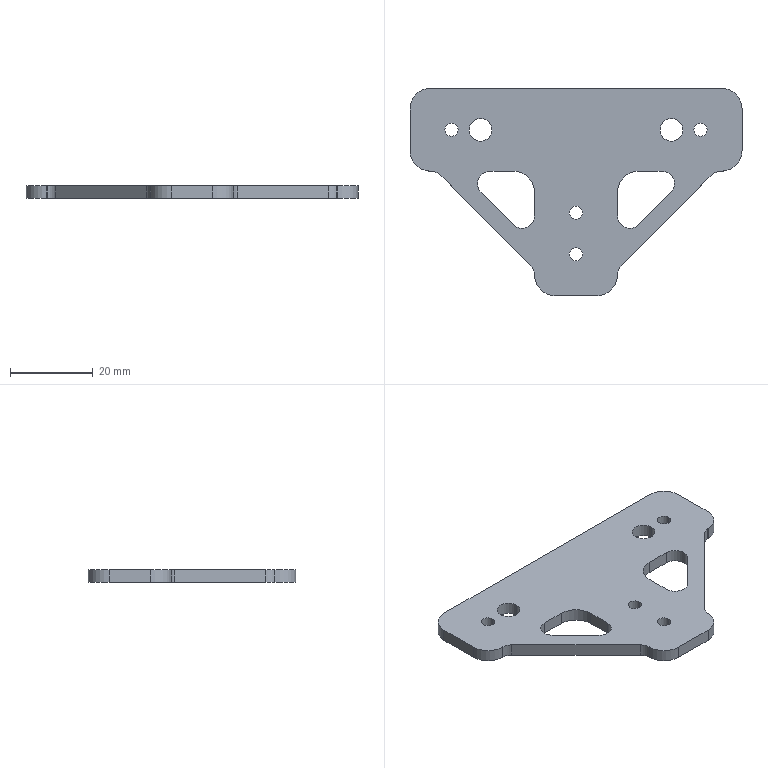Part | SolidWorks | features BaseBody 1 | 1 solid | 47 faces | box 80 x 50 x 3 mm | volume 7139 mm3 | cylinder 29 | plane 18 | commonest cylinder face diameters 6 x9 3.2 x8 10 x8 5.5 x4
STEP:
#1=CARTESIAN_POINT('',(28.4,10.,3.));
#2=VERTEX_POINT('',#1);
#3=CARTESIAN_POINT('',(31.6,10.,3.));
#4=VERTEX_POINT('',#3);
#5=CARTESIAN_POINT('',(30.,10.,3.));
#6=DIRECTION('',(0.,0.,1.));
#7=DIRECTION('',(-1.,0.,0.));
#8=AXIS2_PLACEMENT_3D('',#5,#6,#7);
#9=CIRCLE('',#8,1.6);
#10=EDGE_CURVE('',#2,#4,#9,.T.);
#11=ORIENTED_EDGE('',*,*,#10,.T.);
#12=CARTESIAN_POINT('',(31.6,10.,0.));
#13=VERTEX_POINT('',#12);
#14=CARTESIAN_POINT('',(31.6,10.,3.));
#15=DIRECTION('',(0.,0.,-1.));
#16=VECTOR('',#15,1000.);
#17=LINE('',#14,#16);
#18=EDGE_CURVE('',#4,#13,#17,.T.);
#19=ORIENTED_EDGE('',*,*,#18,.T.);
#20=CARTESIAN_POINT('',(28.4,10.,0.));
#21=VERTEX_POINT('',#20);
#22=CARTESIAN_POINT('',(30.,10.,0.));
#23=DIRECTION('',(0.,0.,1.));
#24=DIRECTION('',(-1.,0.,0.));
#25=AXIS2_PLACEMENT_3D('',#22,#23,#24);
#26=CIRCLE('',#25,1.6);
#27=EDGE_CURVE('',#21,#13,#26,.T.);
#28=ORIENTED_EDGE('',*,*,#27,.F.);
#29=CARTESIAN_POINT('',(28.4,10.,3.));
#30=DIRECTION('',(0.,0.,-1.));
#31=VECTOR('',#30,1000.);
#32=LINE('',#29,#31);
#33=EDGE_CURVE('',#2,#21,#32,.T.);
#34=ORIENTED_EDGE('',*,*,#33,.F.);
#35=EDGE_LOOP('',(#11,#19,#28,#34));
#36=FACE_OUTER_BOUND('',#35,.T.);
#37=CARTESIAN_POINT('',(30.,10.,3.));
#38=DIRECTION('',(0.,0.,-1.));
#39=DIRECTION('',(-1.,0.,0.));
#40=AXIS2_PLACEMENT_3D('',#37,#38,#39);
#41=CYLINDRICAL_SURFACE('',#40,1.6);
#42=ADVANCED_FACE('',(#36),#41,.F.);
#43=CARTESIAN_POINT('',(-25.75,10.,3.));
#44=VERTEX_POINT('',#43);
#45=CARTESIAN_POINT('',(-20.25,10.,3.));
#46=VERTEX_POINT('',#45);
#47=CARTESIAN_POINT('',(-23.,10.,3.));
#48=DIRECTION('',(0.,0.,1.));
#49=DIRECTION('',(-1.,0.,0.));
#50=AXIS2_PLACEMENT_3D('',#47,#48,#49);
#51=CIRCLE('',#50,2.75);
#52=EDGE_CURVE('',#44,#46,#51,.T.);
#53=ORIENTED_EDGE('',*,*,#52,.T.);
#54=CARTESIAN_POINT('',(-20.25,10.,0.));
#55=VERTEX_POINT('',#54);
#56=CARTESIAN_POINT('',(-20.25,10.,3.));
#57=DIRECTION('',(0.,0.,-1.));
#58=VECTOR('',#57,1000.);
#59=LINE('',#56,#58);
#60=EDGE_CURVE('',#46,#55,#59,.T.);
#61=ORIENTED_EDGE('',*,*,#60,.T.);
#62=CARTESIAN_POINT('',(-25.75,10.,0.));
#63=VERTEX_POINT('',#62);
#64=CARTESIAN_POINT('',(-23.,10.,0.));
#65=DIRECTION('',(0.,0.,1.));
#66=DIRECTION('',(-1.,0.,0.));
#67=AXIS2_PLACEMENT_3D('',#64,#65,#66);
#68=CIRCLE('',#67,2.75);
#69=EDGE_CURVE('',#63,#55,#68,.T.);
#70=ORIENTED_EDGE('',*,*,#69,.F.);
#71=CARTESIAN_POINT('',(-25.75,10.,3.));
#72=DIRECTION('',(0.,0.,-1.));
#73=VECTOR('',#72,1000.);
#74=LINE('',#71,#73);
#75=EDGE_CURVE('',#44,#63,#74,.T.);
#76=ORIENTED_EDGE('',*,*,#75,.F.);
#77=EDGE_LOOP('',(#53,#61,#70,#76));
#78=FACE_OUTER_BOUND('',#77,.T.);
#79=CARTESIAN_POINT('',(-23.,10.,3.));
#80=DIRECTION('',(0.,0.,-1.));
#81=DIRECTION('',(-1.,0.,0.));
#82=AXIS2_PLACEMENT_3D('',#79,#80,#81);
#83=CYLINDRICAL_SURFACE('',#82,2.75);
#84=ADVANCED_FACE('',(#78),#83,.F.);
#85=CARTESIAN_POINT('',(-1.6,-20.,3.));
#86=VERTEX_POINT('',#85);
#87=CARTESIAN_POINT('',(1.6,-20.,3.));
#88=VERTEX_POINT('',#87);
#89=CARTESIAN_POINT('',(0.,-20.,3.));
#90=DIRECTION('',(0.,0.,1.));
#91=DIRECTION('',(-1.,0.,0.));
#92=AXIS2_PLACEMENT_3D('',#89,#90,#91);
#93=CIRCLE('',#92,1.6);
#94=EDGE_CURVE('',#86,#88,#93,.T.);
#95=ORIENTED_EDGE('',*,*,#94,.T.);
#96=CARTESIAN_POINT('',(1.6,-20.,0.));
#97=VERTEX_POINT('',#96);
#98=CARTESIAN_POINT('',(1.6,-20.,3.));
#99=DIRECTION('',(0.,0.,-1.));
#100=VECTOR('',#99,1000.);
#101=LINE('',#98,#100);
#102=EDGE_CURVE('',#88,#97,#101,.T.);
#103=ORIENTED_EDGE('',*,*,#102,.T.);
#104=CARTESIAN_POINT('',(-1.6,-20.,0.));
#105=VERTEX_POINT('',#104);
#106=CARTESIAN_POINT('',(0.,-20.,0.));
#107=DIRECTION('',(0.,0.,1.));
#108=DIRECTION('',(-1.,0.,0.));
#109=AXIS2_PLACEMENT_3D('',#106,#107,#108);
#110=CIRCLE('',#109,1.6);
#111=EDGE_CURVE('',#105,#97,#110,.T.);
#112=ORIENTED_EDGE('',*,*,#111,.F.);
#113=CARTESIAN_POINT('',(-1.6,-20.,3.));
#114=DIRECTION('',(0.,0.,-1.));
#115=VECTOR('',#114,1000.);
#116=LINE('',#113,#115);
#117=EDGE_CURVE('',#86,#105,#116,.T.);
#118=ORIENTED_EDGE('',*,*,#117,.F.);
#119=EDGE_LOOP('',(#95,#103,#112,#118));
#120=FACE_OUTER_BOUND('',#119,.T.);
#121=CARTESIAN_POINT('',(0.,-20.,3.));
#122=DIRECTION('',(0.,0.,-1.));
#123=DIRECTION('',(-1.,0.,0.));
#124=AXIS2_PLACEMENT_3D('',#121,#122,#123);
#125=CYLINDRICAL_SURFACE('',#124,1.6);
#126=ADVANCED_FACE('',(#120),#125,.F.);
#127=CARTESIAN_POINT('',(-1.6,-10.,3.));
#128=VERTEX_POINT('',#127);
#129=CARTESIAN_POINT('',(1.6,-10.,3.));
#130=VERTEX_POINT('',#129);
#131=CARTESIAN_POINT('',(0.,-10.,3.));
#132=DIRECTION('',(0.,0.,1.));
#133=DIRECTION('',(-1.,0.,0.));
#134=AXIS2_PLACEMENT_3D('',#131,#132,#133);
#135=CIRCLE('',#134,1.6);
#136=EDGE_CURVE('',#128,#130,#135,.T.);
#137=ORIENTED_EDGE('',*,*,#136,.T.);
#138=CARTESIAN_POINT('',(1.6,-10.,0.));
#139=VERTEX_POINT('',#138);
#140=CARTESIAN_POINT('',(1.6,-10.,3.));
#141=DIRECTION('',(0.,0.,-1.));
#142=VECTOR('',#141,1000.);
#143=LINE('',#140,#142);
#144=EDGE_CURVE('',#130,#139,#143,.T.);
#145=ORIENTED_EDGE('',*,*,#144,.T.);
#146=CARTESIAN_POINT('',(-1.6,-10.,0.));
#147=VERTEX_POINT('',#146);
#148=CARTESIAN_POINT('',(0.,-10.,0.));
#149=DIRECTION('',(0.,0.,1.));
#150=DIRECTION('',(-1.,0.,0.));
#151=AXIS2_PLACEMENT_3D('',#148,#149,#150);
#152=CIRCLE('',#151,1.6);
#153=EDGE_CURVE('',#147,#139,#152,.T.);
#154=ORIENTED_EDGE('',*,*,#153,.F.);
#155=CARTESIAN_POINT('',(-1.6,-10.,3.));
#156=DIRECTION('',(0.,0.,-1.));
#157=VECTOR('',#156,1000.);
#158=LINE('',#155,#157);
#159=EDGE_CURVE('',#128,#147,#158,.T.);
#160=ORIENTED_EDGE('',*,*,#159,.F.);
#161=EDGE_LOOP('',(#137,#145,#154,#160));
#162=FACE_OUTER_BOUND('',#161,.T.);
#163=CARTESIAN_POINT('',(0.,-10.,3.));
#164=DIRECTION('',(0.,0.,-1.));
#165=DIRECTION('',(-1.,0.,0.));
#166=AXIS2_PLACEMENT_3D('',#163,#164,#165);
#167=CYLINDRICAL_SURFACE('',#166,1.6);
#168=ADVANCED_FACE('',(#162),#167,.F.);
#169=CARTESIAN_POINT('',(20.25,10.,3.));
#170=VERTEX_POINT('',#169);
#171=CARTESIAN_POINT('',(25.75,10.,3.));
#172=VERTEX_POINT('',#171);
#173=CARTESIAN_POINT('',(23.,10.,3.));
#174=DIRECTION('',(0.,0.,1.));
#175=DIRECTION('',(-1.,0.,0.));
#176=AXIS2_PLACEMENT_3D('',#173,#174,#175);
#177=CIRCLE('',#176,2.75);
#178=EDGE_CURVE('',#170,#172,#177,.T.);
#179=ORIENTED_EDGE('',*,*,#178,.T.);
#180=CARTESIAN_POINT('',(25.75,10.,0.));
#181=VERTEX_POINT('',#180);
#182=CARTESIAN_POINT('',(25.75,10.,3.));
#183=DIRECTION('',(0.,0.,-1.));
#184=VECTOR('',#183,1000.);
#185=LINE('',#182,#184);
#186=EDGE_CURVE('',#172,#181,#185,.T.);
#187=ORIENTED_EDGE('',*,*,#186,.T.);
#188=CARTESIAN_POINT('',(20.25,10.,0.));
#189=VERTEX_POINT('',#188);
#190=CARTESIAN_POINT('',(23.,10.,0.));
#191=DIRECTION('',(0.,0.,1.));
#192=DIRECTION('',(-1.,0.,0.));
#193=AXIS2_PLACEMENT_3D('',#190,#191,#192);
#194=CIRCLE('',#193,2.75);
#195=EDGE_CURVE('',#189,#181,#194,.T.);
#196=ORIENTED_EDGE('',*,*,#195,.F.);
#197=CARTESIAN_POINT('',(20.25,10.,3.));
#198=DIRECTION('',(0.,0.,-1.));
#199=VECTOR('',#198,1000.);
#200=LINE('',#197,#199);
#201=EDGE_CURVE('',#170,#189,#200,.T.);
#202=ORIENTED_EDGE('',*,*,#201,.F.);
#203=EDGE_LOOP('',(#179,#187,#196,#202));
#204=FACE_OUTER_BOUND('',#203,.T.);
#205=CARTESIAN_POINT('',(23.,10.,3.));
#206=DIRECTION('',(0.,0.,-1.));
#207=DIRECTION('',(-1.,0.,0.));
#208=AXIS2_PLACEMENT_3D('',#205,#206,#207);
#209=CYLINDRICAL_SURFACE('',#208,2.75);
#210=ADVANCED_FACE('',(#204),#209,.F.);
#211=CARTESIAN_POINT('',(-31.6,10.,3.));
#212=VERTEX_POINT('',#211);
#213=CARTESIAN_POINT('',(-28.4,10.,3.));
#214=VERTEX_POINT('',#213);
#215=CARTESIAN_POINT('',(-30.,10.,3.));
#216=DIRECTION('',(0.,0.,1.));
#217=DIRECTION('',(-1.,0.,0.));
#218=AXIS2_PLACEMENT_3D('',#215,#216,#217);
#219=CIRCLE('',#218,1.6);
#220=EDGE_CURVE('',#212,#214,#219,.T.);
#221=ORIENTED_EDGE('',*,*,#220,.T.);
#222=CARTESIAN_POINT('',(-28.4,10.,0.));
#223=VERTEX_POINT('',#222);
#224=CARTESIAN_POINT('',(-28.4,10.,3.));
#225=DIRECTION('',(0.,0.,-1.));
#226=VECTOR('',#225,1000.);
#227=LINE('',#224,#226);
#228=EDGE_CURVE('',#214,#223,#227,.T.);
#229=ORIENTED_EDGE('',*,*,#228,.T.);
#230=CARTESIAN_POINT('',(-31.6,10.,0.));
#231=VERTEX_POINT('',#230);
#232=CARTESIAN_POINT('',(-30.,10.,0.));
#233=DIRECTION('',(0.,0.,1.));
#234=DIRECTION('',(-1.,0.,0.));
#235=AXIS2_PLACEMENT_3D('',#232,#233,#234);
#236=CIRCLE('',#235,1.6);
#237=EDGE_CURVE('',#231,#223,#236,.T.);
#238=ORIENTED_EDGE('',*,*,#237,.F.);
#239=CARTESIAN_POINT('',(-31.6,10.,3.));
#240=DIRECTION('',(0.,0.,-1.));
#241=VECTOR('',#240,1000.);
#242=LINE('',#239,#241);
#243=EDGE_CURVE('',#212,#231,#242,.T.);
#244=ORIENTED_EDGE('',*,*,#243,.F.);
#245=EDGE_LOOP('',(#221,#229,#238,#244));
#246=FACE_OUTER_BOUND('',#245,.T.);
#247=CARTESIAN_POINT('',(-30.,10.,3.));
#248=DIRECTION('',(0.,0.,-1.));
#249=DIRECTION('',(-1.,0.,0.));
#250=AXIS2_PLACEMENT_3D('',#247,#248,#249);
#251=CYLINDRICAL_SURFACE('',#250,1.6);
#252=ADVANCED_FACE('',(#246),#251,.F.);
#253=CARTESIAN_POINT('',(-20.757,0.,3.));
#254=VERTEX_POINT('',#253);
#255=CARTESIAN_POINT('',(-23.757,-3.,3.));
#256=VERTEX_POINT('',#255);
#257=CARTESIAN_POINT('',(-20.757,-3.,3.));
#258=DIRECTION('',(0.,0.,1.));
#259=DIRECTION('',(-1.,0.,0.));
#260=AXIS2_PLACEMENT_3D('',#257,#258,#259);
#261=CIRCLE('',#260,3.);
#262=EDGE_CURVE('',#254,#256,#261,.T.);
#263=ORIENTED_EDGE('',*,*,#262,.T.);
#264=CARTESIAN_POINT('',(-23.757,-3.,0.));
#265=VERTEX_POINT('',#264);
#266=CARTESIAN_POINT('',(-23.757,-3.,3.));
#267=DIRECTION('',(0.,0.,-1.));
#268=VECTOR('',#267,1000.);
#269=LINE('',#266,#268);
#270=EDGE_CURVE('',#256,#265,#269,.T.);
#271=ORIENTED_EDGE('',*,*,#270,.T.);
#272=CARTESIAN_POINT('',(-20.757,0.,0.));
#273=VERTEX_POINT('',#272);
#274=CARTESIAN_POINT('',(-20.757,-3.,0.));
#275=DIRECTION('',(0.,0.,1.));
#276=DIRECTION('',(-1.,0.,0.));
#277=AXIS2_PLACEMENT_3D('',#274,#275,#276);
#278=CIRCLE('',#277,3.);
#279=EDGE_CURVE('',#273,#265,#278,.T.);
#280=ORIENTED_EDGE('',*,*,#279,.F.);
#281=CARTESIAN_POINT('',(-20.757,0.,3.));
#282=DIRECTION('',(0.,0.,-1.));
#283=VECTOR('',#282,1000.);
#284=LINE('',#281,#283);
#285=EDGE_CURVE('',#254,#273,#284,.T.);
#286=ORIENTED_EDGE('',*,*,#285,.F.);
#287=EDGE_LOOP('',(#263,#271,#280,#286));
#288=FACE_OUTER_BOUND('',#287,.T.);
#289=CARTESIAN_POINT('',(-20.757,-3.,3.));
#290=DIRECTION('',(0.,0.,-1.));
#291=DIRECTION('',(-1.,0.,0.));
#292=AXIS2_PLACEMENT_3D('',#289,#290,#291);
#293=CYLINDRICAL_SURFACE('',#292,3.);
#294=ADVANCED_FACE('',(#288),#293,.F.);
#295=ORIENTED_EDGE('',*,*,#10,.F.);
#296=CARTESIAN_POINT('',(30.,10.,3.));
#297=DIRECTION('',(0.,0.,1.));
#298=DIRECTION('',(-1.,0.,0.));
#299=AXIS2_PLACEMENT_3D('',#296,#297,#298);
#300=CIRCLE('',#299,1.6);
#301=EDGE_CURVE('',#4,#2,#300,.T.);
#302=ORIENTED_EDGE('',*,*,#301,.F.);
#303=EDGE_LOOP('',(#295,#302));
#304=FACE_BOUND('',#303,.T.);
#305=ORIENTED_EDGE('',*,*,#52,.F.);
#306=CARTESIAN_POINT('',(-23.,10.,3.));
#307=DIRECTION('',(0.,0.,1.));
#308=DIRECTION('',(-1.,0.,0.));
#309=AXIS2_PLACEMENT_3D('',#306,#307,#308);
#310=CIRCLE('',#309,2.75);
#311=EDGE_CURVE('',#46,#44,#310,.T.);
#312=ORIENTED_EDGE('',*,*,#311,.F.);
#313=EDGE_LOOP('',(#305,#312));
#314=FACE_BOUND('',#313,.T.);
#315=ORIENTED_EDGE('',*,*,#94,.F.);
#316=CARTESIAN_POINT('',(0.,-20.,3.));
#317=DIRECTION('',(0.,0.,1.));
#318=DIRECTION('',(-1.,0.,0.));
#319=AXIS2_PLACEMENT_3D('',#316,#317,#318);
#320=CIRCLE('',#319,1.6);
#321=EDGE_CURVE('',#88,#86,#320,.T.);
#322=ORIENTED_EDGE('',*,*,#321,.F.);
#323=EDGE_LOOP('',(#315,#322));
#324=FACE_BOUND('',#323,.T.);
#325=ORIENTED_EDGE('',*,*,#136,.F.);
#326=CARTESIAN_POINT('',(0.,-10.,3.));
#327=DIRECTION('',(0.,0.,1.));
#328=DIRECTION('',(-1.,0.,0.));
#329=AXIS2_PLACEMENT_3D('',#326,#327,#328);
#330=CIRCLE('',#329,1.6);
#331=EDGE_CURVE('',#130,#128,#330,.T.);
#332=ORIENTED_EDGE('',*,*,#331,.F.);
#333=EDGE_LOOP('',(#325,#332));
#334=FACE_BOUND('',#333,.T.);
#335=ORIENTED_EDGE('',*,*,#178,.F.);
#336=CARTESIAN_POINT('',(23.,10.,3.));
#337=DIRECTION('',(0.,0.,1.));
#338=DIRECTION('',(-1.,0.,0.));
#339=AXIS2_PLACEMENT_3D('',#336,#337,#338);
#340=CIRCLE('',#339,2.75);
#341=EDGE_CURVE('',#172,#170,#340,.T.);
#342=ORIENTED_EDGE('',*,*,#341,.F.);
#343=EDGE_LOOP('',(#335,#342));
#344=FACE_BOUND('',#343,.T.);
#345=ORIENTED_EDGE('',*,*,#220,.F.);
#346=CARTESIAN_POINT('',(-30.,10.,3.));
#347=DIRECTION('',(0.,0.,1.));
#348=DIRECTION('',(-1.,0.,0.));
#349=AXIS2_PLACEMENT_3D('',#346,#347,#348);
#350=CIRCLE('',#349,1.6);
#351=EDGE_CURVE('',#214,#212,#350,.T.);
#352=ORIENTED_EDGE('',*,*,#351,.F.);
#353=EDGE_LOOP('',(#345,#352));
#354=FACE_BOUND('',#353,.T.);
#355=CARTESIAN_POINT('',(-32.778,-0.8787,3.));
#356=VERTEX_POINT('',#355);
#357=CARTESIAN_POINT('',(-34.899,0.,3.));
#358=VERTEX_POINT('',#357);
#359=CARTESIAN_POINT('',(-34.899,-3.,3.));
#360=DIRECTION('',(0.,0.,1.));
#361=DIRECTION('',(-1.,0.,0.));
#362=AXIS2_PLACEMENT_3D('',#359,#360,#361);
#363=CIRCLE('',#362,3.);
#364=EDGE_CURVE('',#356,#358,#363,.T.);
#365=ORIENTED_EDGE('',*,*,#364,.F.);
#366=CARTESIAN_POINT('',(-10.879,-22.778,3.));
#367=VERTEX_POINT('',#366);
#368=CARTESIAN_POINT('',(-10.879,-22.778,3.));
#369=DIRECTION('',(-0.7071,0.7071,0.));
#370=VECTOR('',#369,1000.);
#371=LINE('',#368,#370);
#372=EDGE_CURVE('',#367,#356,#371,.T.);
#373=ORIENTED_EDGE('',*,*,#372,.F.);
#374=CARTESIAN_POINT('',(-10.,-24.899,3.));
#375=VERTEX_POINT('',#374);
#376=CARTESIAN_POINT('',(-13.,-24.899,3.));
#377=DIRECTION('',(0.,0.,1.));
#378=DIRECTION('',(-1.,0.,0.));
#379=AXIS2_PLACEMENT_3D('',#376,#377,#378);
#380=CIRCLE('',#379,3.);
#381=EDGE_CURVE('',#375,#367,#380,.T.);
#382=ORIENTED_EDGE('',*,*,#381,.F.);
#383=CARTESIAN_POINT('',(-10.,-25.,3.));
#384=VERTEX_POINT('',#383);
#385=CARTESIAN_POINT('',(-10.,-30.,3.));
#386=DIRECTION('',(0.,-1.,0.));
#387=VECTOR('',#386,1000.);
#388=LINE('',#385,#387);
#389=EDGE_CURVE('',#375,#384,#388,.T.);
#390=ORIENTED_EDGE('',*,*,#389,.T.);
#391=CARTESIAN_POINT('',(-5.,-30.,3.));
#392=VERTEX_POINT('',#391);
#393=CARTESIAN_POINT('',(-5.,-25.,3.));
#394=DIRECTION('',(0.,0.,-1.));
#395=DIRECTION('',(-1.,0.,0.));
#396=AXIS2_PLACEMENT_3D('',#393,#394,#395);
#397=CIRCLE('',#396,5.);
#398=EDGE_CURVE('',#392,#384,#397,.T.);
#399=ORIENTED_EDGE('',*,*,#398,.F.);
#400=CARTESIAN_POINT('',(5.,-30.,3.));
#401=VERTEX_POINT('',#400);
#402=CARTESIAN_POINT('',(0.,-30.,3.));
#403=DIRECTION('',(-1.,0.,0.));
#404=VECTOR('',#403,1000.);
#405=LINE('',#402,#404);
#406=EDGE_CURVE('',#401,#392,#405,.T.);
#407=ORIENTED_EDGE('',*,*,#406,.F.);
#408=CARTESIAN_POINT('',(10.,-25.,3.));
#409=VERTEX_POINT('',#408);
#410=CARTESIAN_POINT('',(5.,-25.,3.));
#411=DIRECTION('',(0.,0.,-1.));
#412=DIRECTION('',(-1.,0.,0.));
#413=AXIS2_PLACEMENT_3D('',#410,#411,#412);
#414=CIRCLE('',#413,5.);
#415=EDGE_CURVE('',#409,#401,#414,.T.);
#416=ORIENTED_EDGE('',*,*,#415,.F.);
#417=CARTESIAN_POINT('',(10.,-24.899,3.));
#418=VERTEX_POINT('',#417);
#419=CARTESIAN_POINT('',(10.,0.,3.));
#420=DIRECTION('',(0.,1.,0.));
#421=VECTOR('',#420,1000.);
#422=LINE('',#419,#421);
#423=EDGE_CURVE('',#409,#418,#422,.T.);
#424=ORIENTED_EDGE('',*,*,#423,.T.);
#425=CARTESIAN_POINT('',(10.879,-22.778,3.));
#426=VERTEX_POINT('',#425);
#427=CARTESIAN_POINT('',(13.,-24.899,3.));
#428=DIRECTION('',(0.,0.,1.));
#429=DIRECTION('',(-1.,0.,0.));
#430=AXIS2_PLACEMENT_3D('',#427,#428,#429);
#431=CIRCLE('',#430,3.);
#432=EDGE_CURVE('',#426,#418,#431,.T.);
#433=ORIENTED_EDGE('',*,*,#432,.F.);
#434=CARTESIAN_POINT('',(32.778,-0.8787,3.));
#435=VERTEX_POINT('',#434);
#436=CARTESIAN_POINT('',(32.778,-0.8787,3.));
#437=DIRECTION('',(-0.7071,-0.7071,0.));
#438=VECTOR('',#437,1000.);
#439=LINE('',#436,#438);
#440=EDGE_CURVE('',#435,#426,#439,.T.);
#441=ORIENTED_EDGE('',*,*,#440,.F.);
#442=CARTESIAN_POINT('',(34.899,0.,3.));
#443=VERTEX_POINT('',#442);
#444=CARTESIAN_POINT('',(34.899,-3.,3.));
#445=DIRECTION('',(0.,0.,1.));
#446=DIRECTION('',(-1.,0.,0.));
#447=AXIS2_PLACEMENT_3D('',#444,#445,#446);
#448=CIRCLE('',#447,3.);
#449=EDGE_CURVE('',#443,#435,#448,.T.);
#450=ORIENTED_EDGE('',*,*,#449,.F.);
#451=CARTESIAN_POINT('',(35.,0.,3.));
#452=VERTEX_POINT('',#451);
#453=CARTESIAN_POINT('',(40.,0.,3.));
#454=DIRECTION('',(1.,0.,0.));
#455=VECTOR('',#454,1000.);
#456=LINE('',#453,#455);
#457=EDGE_CURVE('',#443,#452,#456,.T.);
#458=ORIENTED_EDGE('',*,*,#457,.T.);
#459=CARTESIAN_POINT('',(40.,5.,3.));
#460=VERTEX_POINT('',#459);
#461=CARTESIAN_POINT('',(35.,5.,3.));
#462=DIRECTION('',(0.,0.,-1.));
#463=DIRECTION('',(-1.,0.,0.));
#464=AXIS2_PLACEMENT_3D('',#461,#462,#463);
#465=CIRCLE('',#464,5.);
#466=EDGE_CURVE('',#460,#452,#465,.T.);
#467=ORIENTED_EDGE('',*,*,#466,.F.);
#468=CARTESIAN_POINT('',(40.,15.,3.));
#469=VERTEX_POINT('',#468);
#470=CARTESIAN_POINT('',(40.,0.,3.));
#471=DIRECTION('',(0.,-1.,0.));
#472=VECTOR('',#471,1000.);
#473=LINE('',#470,#472);
#474=EDGE_CURVE('',#469,#460,#473,.T.);
#475=ORIENTED_EDGE('',*,*,#474,.F.);
#476=CARTESIAN_POINT('',(35.,20.,3.));
#477=VERTEX_POINT('',#476);
#478=CARTESIAN_POINT('',(35.,15.,3.));
#479=DIRECTION('',(0.,0.,-1.));
#480=DIRECTION('',(-1.,0.,0.));
#481=AXIS2_PLACEMENT_3D('',#478,#479,#480);
#482=CIRCLE('',#481,5.);
#483=EDGE_CURVE('',#477,#469,#482,.T.);
#484=ORIENTED_EDGE('',*,*,#483,.F.);
#485=CARTESIAN_POINT('',(-35.,20.,3.));
#486=VERTEX_POINT('',#485);
#487=CARTESIAN_POINT('',(0.,20.,3.));
#488=DIRECTION('',(1.,0.,0.));
#489=VECTOR('',#488,1000.);
#490=LINE('',#487,#489);
#491=EDGE_CURVE('',#486,#477,#490,.T.);
#492=ORIENTED_EDGE('',*,*,#491,.F.);
#493=CARTESIAN_POINT('',(-40.,15.,3.));
#494=VERTEX_POINT('',#493);
#495=CARTESIAN_POINT('',(-35.,15.,3.));
#496=DIRECTION('',(0.,0.,-1.));
#497=DIRECTION('',(-1.,0.,0.));
#498=AXIS2_PLACEMENT_3D('',#495,#496,#497);
#499=CIRCLE('',#498,5.);
#500=EDGE_CURVE('',#494,#486,#499,.T.);
#501=ORIENTED_EDGE('',*,*,#500,.F.);
#502=CARTESIAN_POINT('',(-40.,5.,3.));
#503=VERTEX_POINT('',#502);
#504=CARTESIAN_POINT('',(-40.,0.,3.));
#505=DIRECTION('',(0.,1.,0.));
#506=VECTOR('',#505,1000.);
#507=LINE('',#504,#506);
#508=EDGE_CURVE('',#503,#494,#507,.T.);
#509=ORIENTED_EDGE('',*,*,#508,.F.);
#510=CARTESIAN_POINT('',(-35.,0.,3.));
#511=VERTEX_POINT('',#510);
#512=CARTESIAN_POINT('',(-35.,5.,3.));
#513=DIRECTION('',(0.,0.,-1.));
#514=DIRECTION('',(-1.,0.,0.));
#515=AXIS2_PLACEMENT_3D('',#512,#513,#514);
#516=CIRCLE('',#515,5.);
#517=EDGE_CURVE('',#511,#503,#516,.T.);
#518=ORIENTED_EDGE('',*,*,#517,.F.);
#519=CARTESIAN_POINT('',(-10.,0.,3.));
#520=DIRECTION('',(1.,0.,0.));
#521=VECTOR('',#520,1000.);
#522=LINE('',#519,#521);
#523=EDGE_CURVE('',#511,#358,#522,.T.);
#524=ORIENTED_EDGE('',*,*,#523,.T.);
#525=EDGE_LOOP('',(#365,#373,#382,#390,#399,#407,#416,#424,#433,#441,#450,#458,#467,#475,#484,#492,#501,#509,#518,#524));
#526=FACE_OUTER_BOUND('',#525,.T.);
#527=CARTESIAN_POINT('',(10.,-10.757,3.));
#528=VERTEX_POINT('',#527);
#529=CARTESIAN_POINT('',(15.121,-12.879,3.));
#530=VERTEX_POINT('',#529);
#531=CARTESIAN_POINT('',(13.,-10.757,3.));
#532=DIRECTION('',(0.,0.,1.));
#533=DIRECTION('',(-1.,0.,0.));
#534=AXIS2_PLACEMENT_3D('',#531,#532,#533);
#535=CIRCLE('',#534,3.);
#536=EDGE_CURVE('',#528,#530,#535,.T.);
#537=ORIENTED_EDGE('',*,*,#536,.F.);
#538=CARTESIAN_POINT('',(10.,-5.,3.));
#539=VERTEX_POINT('',#538);
#540=CARTESIAN_POINT('',(10.,0.,3.));
#541=DIRECTION('',(0.,-1.,0.));
#542=VECTOR('',#541,1000.);
#543=LINE('',#540,#542);
#544=EDGE_CURVE('',#539,#528,#543,.T.);
#545=ORIENTED_EDGE('',*,*,#544,.F.);
#546=CARTESIAN_POINT('',(15.,0.,3.));
#547=VERTEX_POINT('',#546);
#548=CARTESIAN_POINT('',(15.,-5.,3.));
#549=DIRECTION('',(0.,0.,1.));
#550=DIRECTION('',(1.,0.,0.));
#551=AXIS2_PLACEMENT_3D('',#548,#549,#550);
#552=CIRCLE('',#551,5.);
#553=EDGE_CURVE('',#547,#539,#552,.T.);
#554=ORIENTED_EDGE('',*,*,#553,.F.);
#555=CARTESIAN_POINT('',(20.757,0.,3.));
#556=VERTEX_POINT('',#555);
#557=CARTESIAN_POINT('',(0.,0.,3.));
#558=DIRECTION('',(-1.,0.,0.));
#559=VECTOR('',#558,1000.);
#560=LINE('',#557,#559);
#561=EDGE_CURVE('',#556,#547,#560,.T.);
#562=ORIENTED_EDGE('',*,*,#561,.F.);
#563=CARTESIAN_POINT('',(22.879,-5.121,3.));
#564=VERTEX_POINT('',#563);
#565=CARTESIAN_POINT('',(20.757,-3.,3.));
#566=DIRECTION('',(0.,0.,1.));
#567=DIRECTION('',(-1.,0.,0.));
#568=AXIS2_PLACEMENT_3D('',#565,#566,#567);
#569=CIRCLE('',#568,3.);
#570=EDGE_CURVE('',#564,#556,#569,.T.);
#571=ORIENTED_EDGE('',*,*,#570,.F.);
#572=CARTESIAN_POINT('',(15.121,-12.879,3.));
#573=DIRECTION('',(0.7071,0.7071,0.));
#574=VECTOR('',#573,1000.);
#575=LINE('',#572,#574);
#576=EDGE_CURVE('',#530,#564,#575,.T.);
#577=ORIENTED_EDGE('',*,*,#576,.F.);
#578=EDGE_LOOP('',(#537,#545,#554,#562,#571,#577));
#579=FACE_BOUND('',#578,.T.);
#580=CARTESIAN_POINT('',(-22.879,-5.121,3.));
#581=VERTEX_POINT('',#580);
#582=CARTESIAN_POINT('',(-15.121,-12.879,3.));
#583=VERTEX_POINT('',#582);
#584=CARTESIAN_POINT('',(-22.879,-5.121,3.));
#585=DIRECTION('',(0.7071,-0.7071,0.));
#586=VECTOR('',#585,1000.);
#587=LINE('',#584,#586);
#588=EDGE_CURVE('',#581,#583,#587,.T.);
#589=ORIENTED_EDGE('',*,*,#588,.F.);
#590=CARTESIAN_POINT('',(-20.757,-3.,3.));
#591=DIRECTION('',(0.,0.,1.));
#592=DIRECTION('',(-1.,0.,0.));
#593=AXIS2_PLACEMENT_3D('',#590,#591,#592);
#594=CIRCLE('',#593,3.);
#595=EDGE_CURVE('',#256,#581,#594,.T.);
#596=ORIENTED_EDGE('',*,*,#595,.F.);
#597=ORIENTED_EDGE('',*,*,#262,.F.);
#598=CARTESIAN_POINT('',(-15.,0.,3.));
#599=VERTEX_POINT('',#598);
#600=CARTESIAN_POINT('',(0.,0.,3.));
#601=DIRECTION('',(-1.,0.,0.));
#602=VECTOR('',#601,1000.);
#603=LINE('',#600,#602);
#604=EDGE_CURVE('',#599,#254,#603,.T.);
#605=ORIENTED_EDGE('',*,*,#604,.F.);
#606=CARTESIAN_POINT('',(-10.,-5.,3.));
#607=VERTEX_POINT('',#606);
#608=CARTESIAN_POINT('',(-15.,-5.,3.));
#609=DIRECTION('',(0.,0.,1.));
#610=DIRECTION('',(1.,0.,0.));
#611=AXIS2_PLACEMENT_3D('',#608,#609,#610);
#612=CIRCLE('',#611,5.);
#613=EDGE_CURVE('',#607,#599,#612,.T.);
#614=ORIENTED_EDGE('',*,*,#613,.F.);
#615=CARTESIAN_POINT('',(-10.,-10.757,3.));
#616=VERTEX_POINT('',#615);
#617=CARTESIAN_POINT('',(-10.,0.,3.));
#618=DIRECTION('',(0.,1.,0.));
#619=VECTOR('',#618,1000.);
#620=LINE('',#617,#619);
#621=EDGE_CURVE('',#616,#607,#620,.T.);
#622=ORIENTED_EDGE('',*,*,#621,.F.);
#623=CARTESIAN_POINT('',(-13.,-10.757,3.));
#624=DIRECTION('',(0.,0.,1.));
#625=DIRECTION('',(-1.,0.,0.));
#626=AXIS2_PLACEMENT_3D('',#623,#624,#625);
#627=CIRCLE('',#626,3.);
#628=EDGE_CURVE('',#583,#616,#627,.T.);
#629=ORIENTED_EDGE('',*,*,#628,.F.);
#630=EDGE_LOOP('',(#589,#596,#597,#605,#614,#622,#629));
#631=FACE_BOUND('',#630,.T.);
#632=CARTESIAN_POINT('',(0.,0.,3.));
#633=DIRECTION('',(0.,0.,-1.));
#634=DIRECTION('',(-1.,0.,0.));
#635=AXIS2_PLACEMENT_3D('',#632,#633,#634);
#636=PLANE('',#635);
#637=ADVANCED_FACE('',(#304,#314,#324,#334,#344,#354,#526,#579,#631),#636,.F.);
#638=ORIENTED_EDGE('',*,*,#18,.F.);
#639=ORIENTED_EDGE('',*,*,#301,.T.);
#640=ORIENTED_EDGE('',*,*,#33,.T.);
#641=CARTESIAN_POINT('',(30.,10.,0.));
#642=DIRECTION('',(0.,0.,1.));
#643=DIRECTION('',(-1.,0.,0.));
#644=AXIS2_PLACEMENT_3D('',#641,#642,#643);
#645=CIRCLE('',#644,1.6);
#646=EDGE_CURVE('',#13,#21,#645,.T.);
#647=ORIENTED_EDGE('',*,*,#646,.F.);
#648=EDGE_LOOP('',(#638,#639,#640,#647));
#649=FACE_OUTER_BOUND('',#648,.T.);
#650=CARTESIAN_POINT('',(30.,10.,3.));
#651=DIRECTION('',(0.,0.,-1.));
#652=DIRECTION('',(-1.,0.,0.));
#653=AXIS2_PLACEMENT_3D('',#650,#651,#652);
#654=CYLINDRICAL_SURFACE('',#653,1.6);
#655=ADVANCED_FACE('',(#649),#654,.F.);
#656=ORIENTED_EDGE('',*,*,#60,.F.);
#657=ORIENTED_EDGE('',*,*,#311,.T.);
#658=ORIENTED_EDGE('',*,*,#75,.T.);
#659=CARTESIAN_POINT('',(-23.,10.,0.));
#660=DIRECTION('',(0.,0.,1.));
#661=DIRECTION('',(-1.,0.,0.));
#662=AXIS2_PLACEMENT_3D('',#659,#660,#661);
#663=CIRCLE('',#662,2.75);
#664=EDGE_CURVE('',#55,#63,#663,.T.);
#665=ORIENTED_EDGE('',*,*,#664,.F.);
#666=EDGE_LOOP('',(#656,#657,#658,#665));
#667=FACE_OUTER_BOUND('',#666,.T.);
#668=CARTESIAN_POINT('',(-23.,10.,3.));
#669=DIRECTION('',(0.,0.,-1.));
#670=DIRECTION('',(-1.,0.,0.));
#671=AXIS2_PLACEMENT_3D('',#668,#669,#670);
#672=CYLINDRICAL_SURFACE('',#671,2.75);
#673=ADVANCED_FACE('',(#667),#672,.F.);
#674=ORIENTED_EDGE('',*,*,#102,.F.);
#675=ORIENTED_EDGE('',*,*,#321,.T.);
#676=ORIENTED_EDGE('',*,*,#117,.T.);
#677=CARTESIAN_POINT('',(0.,-20.,0.));
#678=DIRECTION('',(0.,0.,1.));
#679=DIRECTION('',(-1.,0.,0.));
#680=AXIS2_PLACEMENT_3D('',#677,#678,#679);
#681=CIRCLE('',#680,1.6);
#682=EDGE_CURVE('',#97,#105,#681,.T.);
#683=ORIENTED_EDGE('',*,*,#682,.F.);
#684=EDGE_LOOP('',(#674,#675,#676,#683));
#685=FACE_OUTER_BOUND('',#684,.T.);
#686=CARTESIAN_POINT('',(0.,-20.,3.));
#687=DIRECTION('',(0.,0.,-1.));
#688=DIRECTION('',(-1.,0.,0.));
#689=AXIS2_PLACEMENT_3D('',#686,#687,#688);
#690=CYLINDRICAL_SURFACE('',#689,1.6);
#691=ADVANCED_FACE('',(#685),#690,.F.);
#692=ORIENTED_EDGE('',*,*,#144,.F.);
#693=ORIENTED_EDGE('',*,*,#331,.T.);
#694=ORIENTED_EDGE('',*,*,#159,.T.);
#695=CARTESIAN_POINT('',(0.,-10.,0.));
#696=DIRECTION('',(0.,0.,1.));
#697=DIRECTION('',(-1.,0.,0.));
#698=AXIS2_PLACEMENT_3D('',#695,#696,#697);
#699=CIRCLE('',#698,1.6);
#700=EDGE_CURVE('',#139,#147,#699,.T.);
#701=ORIENTED_EDGE('',*,*,#700,.F.);
#702=EDGE_LOOP('',(#692,#693,#694,#701));
#703=FACE_OUTER_BOUND('',#702,.T.);
#704=CARTESIAN_POINT('',(0.,-10.,3.));
#705=DIRECTION('',(0.,0.,-1.));
#706=DIRECTION('',(-1.,0.,0.));
#707=AXIS2_PLACEMENT_3D('',#704,#705,#706);
#708=CYLINDRICAL_SURFACE('',#707,1.6);
#709=ADVANCED_FACE('',(#703),#708,.F.);
#710=ORIENTED_EDGE('',*,*,#186,.F.);
#711=ORIENTED_EDGE('',*,*,#341,.T.);
#712=ORIENTED_EDGE('',*,*,#201,.T.);
#713=CARTESIAN_POINT('',(23.,10.,0.));
#714=DIRECTION('',(0.,0.,1.));
#715=DIRECTION('',(-1.,0.,0.));
#716=AXIS2_PLACEMENT_3D('',#713,#714,#715);
#717=CIRCLE('',#716,2.75);
#718=EDGE_CURVE('',#181,#189,#717,.T.);
#719=ORIENTED_EDGE('',*,*,#718,.F.);
#720=EDGE_LOOP('',(#710,#711,#712,#719));
#721=FACE_OUTER_BOUND('',#720,.T.);
#722=CARTESIAN_POINT('',(23.,10.,3.));
#723=DIRECTION('',(0.,0.,-1.));
#724=DIRECTION('',(-1.,0.,0.));
#725=AXIS2_PLACEMENT_3D('',#722,#723,#724);
#726=CYLINDRICAL_SURFACE('',#725,2.75);
#727=ADVANCED_FACE('',(#721),#726,.F.);
#728=ORIENTED_EDGE('',*,*,#228,.F.);
#729=ORIENTED_EDGE('',*,*,#351,.T.);
#730=ORIENTED_EDGE('',*,*,#243,.T.);
#731=CARTESIAN_POINT('',(-30.,10.,0.));
#732=DIRECTION('',(0.,0.,1.));
#733=DIRECTION('',(-1.,0.,0.));
#734=AXIS2_PLACEMENT_3D('',#731,#732,#733);
#735=CIRCLE('',#734,1.6);
#736=EDGE_CURVE('',#223,#231,#735,.T.);
#737=ORIENTED_EDGE('',*,*,#736,.F.);
#738=EDGE_LOOP('',(#728,#729,#730,#737));
#739=FACE_OUTER_BOUND('',#738,.T.);
#740=CARTESIAN_POINT('',(-30.,10.,3.));
#741=DIRECTION('',(0.,0.,-1.));
#742=DIRECTION('',(-1.,0.,0.));
#743=AXIS2_PLACEMENT_3D('',#740,#741,#742);
#744=CYLINDRICAL_SURFACE('',#743,1.6);
#745=ADVANCED_FACE('',(#739),#744,.F.);
#746=CARTESIAN_POINT('',(-34.899,0.,0.));
#747=VERTEX_POINT('',#746);
#748=CARTESIAN_POINT('',(-34.899,0.,3.));
#749=DIRECTION('',(0.,0.,1.));
#750=VECTOR('',#749,1000.);
#751=LINE('',#748,#750);
#752=EDGE_CURVE('',#747,#358,#751,.T.);
#753=ORIENTED_EDGE('',*,*,#752,.F.);
#754=CARTESIAN_POINT('',(-32.778,-0.8787,0.));
#755=VERTEX_POINT('',#754);
#756=CARTESIAN_POINT('',(-34.899,-3.,0.));
#757=DIRECTION('',(0.,0.,1.));
#758=DIRECTION('',(-1.,0.,0.));
#759=AXIS2_PLACEMENT_3D('',#756,#757,#758);
#760=CIRCLE('',#759,3.);
#761=EDGE_CURVE('',#755,#747,#760,.T.);
#762=ORIENTED_EDGE('',*,*,#761,.F.);
#763=CARTESIAN_POINT('',(-32.778,-0.8787,3.));
#764=DIRECTION('',(0.,0.,-1.));
#765=VECTOR('',#764,1000.);
#766=LINE('',#763,#765);
#767=EDGE_CURVE('',#356,#755,#766,.T.);
#768=ORIENTED_EDGE('',*,*,#767,.F.);
#769=ORIENTED_EDGE('',*,*,#364,.T.);
#770=EDGE_LOOP('',(#753,#762,#768,#769));
#771=FACE_OUTER_BOUND('',#770,.T.);
#772=CARTESIAN_POINT('',(-34.899,-3.,3.));
#773=DIRECTION('',(0.,0.,-1.));
#774=DIRECTION('',(-1.,0.,0.));
#775=AXIS2_PLACEMENT_3D('',#772,#773,#774);
#776=CYLINDRICAL_SURFACE('',#775,3.);
#777=ADVANCED_FACE('',(#771),#776,.F.);
#778=ORIENTED_EDGE('',*,*,#372,.T.);
#779=ORIENTED_EDGE('',*,*,#767,.T.);
#780=CARTESIAN_POINT('',(-10.879,-22.778,0.));
#781=VERTEX_POINT('',#780);
#782=CARTESIAN_POINT('',(-33.657,0.,0.));
#783=DIRECTION('',(0.7071,-0.7071,0.));
#784=VECTOR('',#783,1000.);
#785=LINE('',#782,#784);
#786=EDGE_CURVE('',#755,#781,#785,.T.);
#787=ORIENTED_EDGE('',*,*,#786,.T.);
#788=CARTESIAN_POINT('',(-10.879,-22.778,3.));
#789=DIRECTION('',(0.,0.,1.));
#790=VECTOR('',#789,1000.);
#791=LINE('',#788,#790);
#792=EDGE_CURVE('',#781,#367,#791,.T.);
#793=ORIENTED_EDGE('',*,*,#792,.T.);
#794=EDGE_LOOP('',(#778,#779,#787,#793));
#795=FACE_OUTER_BOUND('',#794,.T.);
#796=CARTESIAN_POINT('',(-33.657,0.,3.));
#797=DIRECTION('',(-0.7071,-0.7071,0.));
#798=DIRECTION('',(0.7071,-0.7071,0.));
#799=AXIS2_PLACEMENT_3D('',#796,#797,#798);
#800=PLANE('',#799);
#801=ADVANCED_FACE('',(#795),#800,.T.);
#802=ORIENTED_EDGE('',*,*,#792,.F.);
#803=CARTESIAN_POINT('',(-10.,-24.899,0.));
#804=VERTEX_POINT('',#803);
#805=CARTESIAN_POINT('',(-13.,-24.899,0.));
#806=DIRECTION('',(0.,0.,1.));
#807=DIRECTION('',(-1.,0.,0.));
#808=AXIS2_PLACEMENT_3D('',#805,#806,#807);
#809=CIRCLE('',#808,3.);
#810=EDGE_CURVE('',#804,#781,#809,.T.);
#811=ORIENTED_EDGE('',*,*,#810,.F.);
#812=CARTESIAN_POINT('',(-10.,-24.899,3.));
#813=DIRECTION('',(0.,0.,-1.));
#814=VECTOR('',#813,1000.);
#815=LINE('',#812,#814);
#816=EDGE_CURVE('',#375,#804,#815,.T.);
#817=ORIENTED_EDGE('',*,*,#816,.F.);
#818=ORIENTED_EDGE('',*,*,#381,.T.);
#819=EDGE_LOOP('',(#802,#811,#817,#818));
#820=FACE_OUTER_BOUND('',#819,.T.);
#821=CARTESIAN_POINT('',(-13.,-24.899,3.));
#822=DIRECTION('',(0.,0.,-1.));
#823=DIRECTION('',(-1.,0.,0.));
#824=AXIS2_PLACEMENT_3D('',#821,#822,#823);
#825=CYLINDRICAL_SURFACE('',#824,3.);
#826=ADVANCED_FACE('',(#820),#825,.F.);
#827=CARTESIAN_POINT('',(-10.,-25.,0.));
#828=VERTEX_POINT('',#827);
#829=CARTESIAN_POINT('',(-5.,-30.,0.));
#830=VERTEX_POINT('',#829);
#831=CARTESIAN_POINT('',(-5.,-25.,0.));
#832=DIRECTION('',(0.,0.,1.));
#833=DIRECTION('',(-1.,0.,0.));
#834=AXIS2_PLACEMENT_3D('',#831,#832,#833);
#835=CIRCLE('',#834,5.);
#836=EDGE_CURVE('',#828,#830,#835,.T.);
#837=ORIENTED_EDGE('',*,*,#836,.T.);
#838=CARTESIAN_POINT('',(-5.,-30.,3.));
#839=DIRECTION('',(0.,0.,1.));
#840=VECTOR('',#839,1000.);
#841=LINE('',#838,#840);
#842=EDGE_CURVE('',#830,#392,#841,.T.);
#843=ORIENTED_EDGE('',*,*,#842,.T.);
#844=ORIENTED_EDGE('',*,*,#398,.T.);
#845=CARTESIAN_POINT('',(-10.,-25.,3.));
#846=DIRECTION('',(0.,0.,-1.));
#847=VECTOR('',#846,1000.);
#848=LINE('',#845,#847);
#849=EDGE_CURVE('',#384,#828,#848,.T.);
#850=ORIENTED_EDGE('',*,*,#849,.T.);
#851=EDGE_LOOP('',(#837,#843,#844,#850));
#852=FACE_OUTER_BOUND('',#851,.T.);
#853=CARTESIAN_POINT('',(-5.,-25.,3.));
#854=DIRECTION('',(0.,0.,-1.));
#855=DIRECTION('',(-1.,0.,0.));
#856=AXIS2_PLACEMENT_3D('',#853,#854,#855);
#857=CYLINDRICAL_SURFACE('',#856,5.);
#858=ADVANCED_FACE('',(#852),#857,.T.);
#859=ORIENTED_EDGE('',*,*,#842,.F.);
#860=CARTESIAN_POINT('',(5.,-30.,0.));
#861=VERTEX_POINT('',#860);
#862=CARTESIAN_POINT('',(10.,-30.,0.));
#863=DIRECTION('',(-1.,0.,0.));
#864=VECTOR('',#863,1000.);
#865=LINE('',#862,#864);
#866=EDGE_CURVE('',#861,#830,#865,.T.);
#867=ORIENTED_EDGE('',*,*,#866,.F.);
#868=CARTESIAN_POINT('',(5.,-30.,3.));
#869=DIRECTION('',(0.,0.,-1.));
#870=VECTOR('',#869,1000.);
#871=LINE('',#868,#870);
#872=EDGE_CURVE('',#401,#861,#871,.T.);
#873=ORIENTED_EDGE('',*,*,#872,.F.);
#874=ORIENTED_EDGE('',*,*,#406,.T.);
#875=EDGE_LOOP('',(#859,#867,#873,#874));
#876=FACE_OUTER_BOUND('',#875,.T.);
#877=CARTESIAN_POINT('',(10.,-30.,3.));
#878=DIRECTION('',(0.,1.,0.));
#879=DIRECTION('',(-1.,0.,0.));
#880=AXIS2_PLACEMENT_3D('',#877,#878,#879);
#881=PLANE('',#880);
#882=ADVANCED_FACE('',(#876),#881,.F.);
#883=CARTESIAN_POINT('',(10.,-25.,0.));
#884=VERTEX_POINT('',#883);
#885=CARTESIAN_POINT('',(5.,-25.,0.));
#886=DIRECTION('',(0.,0.,1.));
#887=DIRECTION('',(-1.,0.,0.));
#888=AXIS2_PLACEMENT_3D('',#885,#886,#887);
#889=CIRCLE('',#888,5.);
#890=EDGE_CURVE('',#861,#884,#889,.T.);
#891=ORIENTED_EDGE('',*,*,#890,.T.);
#892=CARTESIAN_POINT('',(10.,-25.,3.));
#893=DIRECTION('',(0.,0.,1.));
#894=VECTOR('',#893,1000.);
#895=LINE('',#892,#894);
#896=EDGE_CURVE('',#884,#409,#895,.T.);
#897=ORIENTED_EDGE('',*,*,#896,.T.);
#898=ORIENTED_EDGE('',*,*,#415,.T.);
#899=ORIENTED_EDGE('',*,*,#872,.T.);
#900=EDGE_LOOP('',(#891,#897,#898,#899));
#901=FACE_OUTER_BOUND('',#900,.T.);
#902=CARTESIAN_POINT('',(5.,-25.,3.));
#903=DIRECTION('',(0.,0.,-1.));
#904=DIRECTION('',(-1.,0.,0.));
#905=AXIS2_PLACEMENT_3D('',#902,#903,#904);
#906=CYLINDRICAL_SURFACE('',#905,5.);
#907=ADVANCED_FACE('',(#901),#906,.T.);
#908=CARTESIAN_POINT('',(10.,-24.899,0.));
#909=VERTEX_POINT('',#908);
#910=CARTESIAN_POINT('',(10.,-24.899,3.));
#911=DIRECTION('',(0.,0.,1.));
#912=VECTOR('',#911,1000.);
#913=LINE('',#910,#912);
#914=EDGE_CURVE('',#909,#418,#913,.T.);
#915=ORIENTED_EDGE('',*,*,#914,.F.);
#916=CARTESIAN_POINT('',(10.879,-22.778,0.));
#917=VERTEX_POINT('',#916);
#918=CARTESIAN_POINT('',(13.,-24.899,0.));
#919=DIRECTION('',(0.,0.,1.));
#920=DIRECTION('',(-1.,0.,0.));
#921=AXIS2_PLACEMENT_3D('',#918,#919,#920);
#922=CIRCLE('',#921,3.);
#923=EDGE_CURVE('',#917,#909,#922,.T.);
#924=ORIENTED_EDGE('',*,*,#923,.F.);
#925=CARTESIAN_POINT('',(10.879,-22.778,3.));
#926=DIRECTION('',(0.,0.,-1.));
#927=VECTOR('',#926,1000.);
#928=LINE('',#925,#927);
#929=EDGE_CURVE('',#426,#917,#928,.T.);
#930=ORIENTED_EDGE('',*,*,#929,.F.);
#931=ORIENTED_EDGE('',*,*,#432,.T.);
#932=EDGE_LOOP('',(#915,#924,#930,#931));
#933=FACE_OUTER_BOUND('',#932,.T.);
#934=CARTESIAN_POINT('',(13.,-24.899,3.));
#935=DIRECTION('',(0.,0.,-1.));
#936=DIRECTION('',(-1.,0.,0.));
#937=AXIS2_PLACEMENT_3D('',#934,#935,#936);
#938=CYLINDRICAL_SURFACE('',#937,3.);
#939=ADVANCED_FACE('',(#933),#938,.F.);
#940=CARTESIAN_POINT('',(32.778,-0.8787,0.));
#941=VERTEX_POINT('',#940);
#942=CARTESIAN_POINT('',(33.657,0.,0.));
#943=DIRECTION('',(0.7071,0.7071,0.));
#944=VECTOR('',#943,1000.);
#945=LINE('',#942,#944);
#946=EDGE_CURVE('',#917,#941,#945,.T.);
#947=ORIENTED_EDGE('',*,*,#946,.T.);
#948=CARTESIAN_POINT('',(32.778,-0.8787,3.));
#949=DIRECTION('',(0.,0.,1.));
#950=VECTOR('',#949,1000.);
#951=LINE('',#948,#950);
#952=EDGE_CURVE('',#941,#435,#951,.T.);
#953=ORIENTED_EDGE('',*,*,#952,.T.);
#954=ORIENTED_EDGE('',*,*,#440,.T.);
#955=ORIENTED_EDGE('',*,*,#929,.T.);
#956=EDGE_LOOP('',(#947,#953,#954,#955));
#957=FACE_OUTER_BOUND('',#956,.T.);
#958=CARTESIAN_POINT('',(33.657,0.,3.));
#959=DIRECTION('',(0.7071,-0.7071,0.));
#960=DIRECTION('',(0.7071,0.7071,0.));
#961=AXIS2_PLACEMENT_3D('',#958,#959,#960);
#962=PLANE('',#961);
#963=ADVANCED_FACE('',(#957),#962,.T.);
#964=ORIENTED_EDGE('',*,*,#952,.F.);
#965=CARTESIAN_POINT('',(34.899,0.,0.));
#966=VERTEX_POINT('',#965);
#967=CARTESIAN_POINT('',(34.899,-3.,0.));
#968=DIRECTION('',(0.,0.,1.));
#969=DIRECTION('',(-1.,0.,0.));
#970=AXIS2_PLACEMENT_3D('',#967,#968,#969);
#971=CIRCLE('',#970,3.);
#972=EDGE_CURVE('',#966,#941,#971,.T.);
#973=ORIENTED_EDGE('',*,*,#972,.F.);
#974=CARTESIAN_POINT('',(34.899,0.,3.));
#975=DIRECTION('',(0.,0.,-1.));
#976=VECTOR('',#975,1000.);
#977=LINE('',#974,#976);
#978=EDGE_CURVE('',#443,#966,#977,.T.);
#979=ORIENTED_EDGE('',*,*,#978,.F.);
#980=ORIENTED_EDGE('',*,*,#449,.T.);
#981=EDGE_LOOP('',(#964,#973,#979,#980));
#982=FACE_OUTER_BOUND('',#981,.T.);
#983=CARTESIAN_POINT('',(34.899,-3.,3.));
#984=DIRECTION('',(0.,0.,-1.));
#985=DIRECTION('',(-1.,0.,0.));
#986=AXIS2_PLACEMENT_3D('',#983,#984,#985);
#987=CYLINDRICAL_SURFACE('',#986,3.);
#988=ADVANCED_FACE('',(#982),#987,.F.);
#989=CARTESIAN_POINT('',(35.,0.,0.));
#990=VERTEX_POINT('',#989);
#991=CARTESIAN_POINT('',(40.,5.,0.));
#992=VERTEX_POINT('',#991);
#993=CARTESIAN_POINT('',(35.,5.,0.));
#994=DIRECTION('',(0.,0.,1.));
#995=DIRECTION('',(-1.,0.,0.));
#996=AXIS2_PLACEMENT_3D('',#993,#994,#995);
#997=CIRCLE('',#996,5.);
#998=EDGE_CURVE('',#990,#992,#997,.T.);
#999=ORIENTED_EDGE('',*,*,#998,.T.);
#1000=CARTESIAN_POINT('',(40.,5.,3.));
#1001=DIRECTION('',(0.,0.,1.));
#1002=VECTOR('',#1001,1000.);
#1003=LINE('',#1000,#1002);
#1004=EDGE_CURVE('',#992,#460,#1003,.T.);
#1005=ORIENTED_EDGE('',*,*,#1004,.T.);
#1006=ORIENTED_EDGE('',*,*,#466,.T.);
#1007=CARTESIAN_POINT('',(35.,0.,3.));
#1008=DIRECTION('',(0.,0.,-1.));
#1009=VECTOR('',#1008,1000.);
#1010=LINE('',#1007,#1009);
#1011=EDGE_CURVE('',#452,#990,#1010,.T.);
#1012=ORIENTED_EDGE('',*,*,#1011,.T.);
#1013=EDGE_LOOP('',(#999,#1005,#1006,#1012));
#1014=FACE_OUTER_BOUND('',#1013,.T.);
#1015=CARTESIAN_POINT('',(35.,5.,3.));
#1016=DIRECTION('',(0.,0.,-1.));
#1017=DIRECTION('',(-1.,0.,0.));
#1018=AXIS2_PLACEMENT_3D('',#1015,#1016,#1017);
#1019=CYLINDRICAL_SURFACE('',#1018,5.);
#1020=ADVANCED_FACE('',(#1014),#1019,.T.);
#1021=CARTESIAN_POINT('',(40.,15.,0.));
#1022=VERTEX_POINT('',#1021);
#1023=CARTESIAN_POINT('',(40.,15.,3.));
#1024=DIRECTION('',(0.,0.,-1.));
#1025=VECTOR('',#1024,1000.);
#1026=LINE('',#1023,#1025);
#1027=EDGE_CURVE('',#469,#1022,#1026,.T.);
#1028=ORIENTED_EDGE('',*,*,#1027,.F.);
#1029=ORIENTED_EDGE('',*,*,#474,.T.);
#1030=ORIENTED_EDGE('',*,*,#1004,.F.);
#1031=CARTESIAN_POINT('',(40.,20.,0.));
#1032=DIRECTION('',(0.,-1.,0.));
#1033=VECTOR('',#1032,1000.);
#1034=LINE('',#1031,#1033);
#1035=EDGE_CURVE('',#1022,#992,#1034,.T.);
#1036=ORIENTED_EDGE('',*,*,#1035,.F.);
#1037=EDGE_LOOP('',(#1028,#1029,#1030,#1036));
#1038=FACE_OUTER_BOUND('',#1037,.T.);
#1039=CARTESIAN_POINT('',(40.,20.,3.));
#1040=DIRECTION('',(-1.,0.,0.));
#1041=DIRECTION('',(0.,0.,1.));
#1042=AXIS2_PLACEMENT_3D('',#1039,#1040,#1041);
#1043=PLANE('',#1042);
#1044=ADVANCED_FACE('',(#1038),#1043,.F.);
#1045=CARTESIAN_POINT('',(35.,20.,0.));
#1046=VERTEX_POINT('',#1045);
#1047=CARTESIAN_POINT('',(35.,15.,0.));
#1048=DIRECTION('',(0.,0.,1.));
#1049=DIRECTION('',(-1.,0.,0.));
#1050=AXIS2_PLACEMENT_3D('',#1047,#1048,#1049);
#1051=CIRCLE('',#1050,5.);
#1052=EDGE_CURVE('',#1022,#1046,#1051,.T.);
#1053=ORIENTED_EDGE('',*,*,#1052,.T.);
#1054=CARTESIAN_POINT('',(35.,20.,3.));
#1055=DIRECTION('',(0.,0.,1.));
#1056=VECTOR('',#1055,1000.);
#1057=LINE('',#1054,#1056);
#1058=EDGE_CURVE('',#1046,#477,#1057,.T.);
#1059=ORIENTED_EDGE('',*,*,#1058,.T.);
#1060=ORIENTED_EDGE('',*,*,#483,.T.);
#1061=ORIENTED_EDGE('',*,*,#1027,.T.);
#1062=EDGE_LOOP('',(#1053,#1059,#1060,#1061));
#1063=FACE_OUTER_BOUND('',#1062,.T.);
#1064=CARTESIAN_POINT('',(35.,15.,3.));
#1065=DIRECTION('',(0.,0.,-1.));
#1066=DIRECTION('',(-1.,0.,0.));
#1067=AXIS2_PLACEMENT_3D('',#1064,#1065,#1066);
#1068=CYLINDRICAL_SURFACE('',#1067,5.);
#1069=ADVANCED_FACE('',(#1063),#1068,.T.);
#1070=ORIENTED_EDGE('',*,*,#1058,.F.);
#1071=CARTESIAN_POINT('',(-35.,20.,0.));
#1072=VERTEX_POINT('',#1071);
#1073=CARTESIAN_POINT('',(-40.,20.,0.));
#1074=DIRECTION('',(1.,0.,0.));
#1075=VECTOR('',#1074,1000.);
#1076=LINE('',#1073,#1075);
#1077=EDGE_CURVE('',#1072,#1046,#1076,.T.);
#1078=ORIENTED_EDGE('',*,*,#1077,.F.);
#1079=CARTESIAN_POINT('',(-35.,20.,3.));
#1080=DIRECTION('',(0.,0.,-1.));
#1081=VECTOR('',#1080,1000.);
#1082=LINE('',#1079,#1081);
#1083=EDGE_CURVE('',#486,#1072,#1082,.T.);
#1084=ORIENTED_EDGE('',*,*,#1083,.F.);
#1085=ORIENTED_EDGE('',*,*,#491,.T.);
#1086=EDGE_LOOP('',(#1070,#1078,#1084,#1085));
#1087=FACE_OUTER_BOUND('',#1086,.T.);
#1088=CARTESIAN_POINT('',(-40.,20.,3.));
#1089=DIRECTION('',(0.,-1.,0.));
#1090=DIRECTION('',(1.,0.,0.));
#1091=AXIS2_PLACEMENT_3D('',#1088,#1089,#1090);
#1092=PLANE('',#1091);
#1093=ADVANCED_FACE('',(#1087),#1092,.F.);
#1094=CARTESIAN_POINT('',(-40.,15.,0.));
#1095=VERTEX_POINT('',#1094);
#1096=CARTESIAN_POINT('',(-35.,15.,0.));
#1097=DIRECTION('',(0.,0.,1.));
#1098=DIRECTION('',(-1.,0.,0.));
#1099=AXIS2_PLACEMENT_3D('',#1096,#1097,#1098);
#1100=CIRCLE('',#1099,5.);
#1101=EDGE_CURVE('',#1072,#1095,#1100,.T.);
#1102=ORIENTED_EDGE('',*,*,#1101,.T.);
#1103=CARTESIAN_POINT('',(-40.,15.,3.));
#1104=DIRECTION('',(0.,0.,1.));
#1105=VECTOR('',#1104,1000.);
#1106=LINE('',#1103,#1105);
#1107=EDGE_CURVE('',#1095,#494,#1106,.T.);
#1108=ORIENTED_EDGE('',*,*,#1107,.T.);
#1109=ORIENTED_EDGE('',*,*,#500,.T.);
#1110=ORIENTED_EDGE('',*,*,#1083,.T.);
#1111=EDGE_LOOP('',(#1102,#1108,#1109,#1110));
#1112=FACE_OUTER_BOUND('',#1111,.T.);
#1113=CARTESIAN_POINT('',(-35.,15.,3.));
#1114=DIRECTION('',(0.,0.,-1.));
#1115=DIRECTION('',(-1.,0.,0.));
#1116=AXIS2_PLACEMENT_3D('',#1113,#1114,#1115);
#1117=CYLINDRICAL_SURFACE('',#1116,5.);
#1118=ADVANCED_FACE('',(#1112),#1117,.T.);
#1119=CARTESIAN_POINT('',(-40.,5.,0.));
#1120=VERTEX_POINT('',#1119);
#1121=CARTESIAN_POINT('',(-40.,5.,3.));
#1122=DIRECTION('',(0.,0.,-1.));
#1123=VECTOR('',#1122,1000.);
#1124=LINE('',#1121,#1123);
#1125=EDGE_CURVE('',#503,#1120,#1124,.T.);
#1126=ORIENTED_EDGE('',*,*,#1125,.F.);
#1127=ORIENTED_EDGE('',*,*,#508,.T.);
#1128=ORIENTED_EDGE('',*,*,#1107,.F.);
#1129=CARTESIAN_POINT('',(-40.,0.,0.));
#1130=DIRECTION('',(0.,1.,0.));
#1131=VECTOR('',#1130,1000.);
#1132=LINE('',#1129,#1131);
#1133=EDGE_CURVE('',#1120,#1095,#1132,.T.);
#1134=ORIENTED_EDGE('',*,*,#1133,.F.);
#1135=EDGE_LOOP('',(#1126,#1127,#1128,#1134));
#1136=FACE_OUTER_BOUND('',#1135,.T.);
#1137=CARTESIAN_POINT('',(-40.,0.,3.));
#1138=DIRECTION('',(1.,0.,0.));
#1139=DIRECTION('',(0.,0.,-1.));
#1140=AXIS2_PLACEMENT_3D('',#1137,#1138,#1139);
#1141=PLANE('',#1140);
#1142=ADVANCED_FACE('',(#1136),#1141,.F.);
#1143=CARTESIAN_POINT('',(-35.,0.,0.));
#1144=VERTEX_POINT('',#1143);
#1145=CARTESIAN_POINT('',(-35.,5.,0.));
#1146=DIRECTION('',(0.,0.,1.));
#1147=DIRECTION('',(-1.,0.,0.));
#1148=AXIS2_PLACEMENT_3D('',#1145,#1146,#1147);
#1149=CIRCLE('',#1148,5.);
#1150=EDGE_CURVE('',#1120,#1144,#1149,.T.);
#1151=ORIENTED_EDGE('',*,*,#1150,.T.);
#1152=CARTESIAN_POINT('',(-35.,0.,3.));
#1153=DIRECTION('',(0.,0.,1.));
#1154=VECTOR('',#1153,1000.);
#1155=LINE('',#1152,#1154);
#1156=EDGE_CURVE('',#1144,#511,#1155,.T.);
#1157=ORIENTED_EDGE('',*,*,#1156,.T.);
#1158=ORIENTED_EDGE('',*,*,#517,.T.);
#1159=ORIENTED_EDGE('',*,*,#1125,.T.);
#1160=EDGE_LOOP('',(#1151,#1157,#1158,#1159));
#1161=FACE_OUTER_BOUND('',#1160,.T.);
#1162=CARTESIAN_POINT('',(-35.,5.,3.));
#1163=DIRECTION('',(0.,0.,-1.));
#1164=DIRECTION('',(-1.,0.,0.));
#1165=AXIS2_PLACEMENT_3D('',#1162,#1163,#1164);
#1166=CYLINDRICAL_SURFACE('',#1165,5.);
#1167=ADVANCED_FACE('',(#1161),#1166,.T.);
#1168=ORIENTED_EDGE('',*,*,#576,.T.);
#1169=CARTESIAN_POINT('',(22.879,-5.121,0.));
#1170=VERTEX_POINT('',#1169);
#1171=CARTESIAN_POINT('',(22.879,-5.121,3.));
#1172=DIRECTION('',(0.,0.,-1.));
#1173=VECTOR('',#1172,1000.);
#1174=LINE('',#1171,#1173);
#1175=EDGE_CURVE('',#564,#1170,#1174,.T.);
#1176=ORIENTED_EDGE('',*,*,#1175,.T.);
#1177=CARTESIAN_POINT('',(15.121,-12.879,0.));
#1178=VERTEX_POINT('',#1177);
#1179=CARTESIAN_POINT('',(10.,-18.,0.));
#1180=DIRECTION('',(-0.7071,-0.7071,0.));
#1181=VECTOR('',#1180,1000.);
#1182=LINE('',#1179,#1181);
#1183=EDGE_CURVE('',#1170,#1178,#1182,.T.);
#1184=ORIENTED_EDGE('',*,*,#1183,.T.);
#1185=CARTESIAN_POINT('',(15.121,-12.879,3.));
#1186=DIRECTION('',(0.,0.,1.));
#1187=VECTOR('',#1186,1000.);
#1188=LINE('',#1185,#1187);
#1189=EDGE_CURVE('',#1178,#530,#1188,.T.);
#1190=ORIENTED_EDGE('',*,*,#1189,.T.);
#1191=EDGE_LOOP('',(#1168,#1176,#1184,#1190));
#1192=FACE_OUTER_BOUND('',#1191,.T.);
#1193=CARTESIAN_POINT('',(10.,-18.,3.));
#1194=DIRECTION('',(-0.7071,0.7071,0.));
#1195=DIRECTION('',(-0.7071,-0.7071,0.));
#1196=AXIS2_PLACEMENT_3D('',#1193,#1194,#1195);
#1197=PLANE('',#1196);
#1198=ADVANCED_FACE('',(#1192),#1197,.T.);
#1199=ORIENTED_EDGE('',*,*,#1189,.F.);
#1200=CARTESIAN_POINT('',(10.,-10.757,0.));
#1201=VERTEX_POINT('',#1200);
#1202=CARTESIAN_POINT('',(13.,-10.757,0.));
#1203=DIRECTION('',(0.,0.,1.));
#1204=DIRECTION('',(-1.,0.,0.));
#1205=AXIS2_PLACEMENT_3D('',#1202,#1203,#1204);
#1206=CIRCLE('',#1205,3.);
#1207=EDGE_CURVE('',#1201,#1178,#1206,.T.);
#1208=ORIENTED_EDGE('',*,*,#1207,.F.);
#1209=CARTESIAN_POINT('',(10.,-10.757,3.));
#1210=DIRECTION('',(0.,0.,-1.));
#1211=VECTOR('',#1210,1000.);
#1212=LINE('',#1209,#1211);
#1213=EDGE_CURVE('',#528,#1201,#1212,.T.);
#1214=ORIENTED_EDGE('',*,*,#1213,.F.);
#1215=ORIENTED_EDGE('',*,*,#536,.T.);
#1216=EDGE_LOOP('',(#1199,#1208,#1214,#1215));
#1217=FACE_OUTER_BOUND('',#1216,.T.);
#1218=CARTESIAN_POINT('',(13.,-10.757,3.));
#1219=DIRECTION('',(0.,0.,-1.));
#1220=DIRECTION('',(-1.,0.,0.));
#1221=AXIS2_PLACEMENT_3D('',#1218,#1219,#1220);
#1222=CYLINDRICAL_SURFACE('',#1221,3.);
#1223=ADVANCED_FACE('',(#1217),#1222,.F.);
#1224=ORIENTED_EDGE('',*,*,#1213,.T.);
#1225=CARTESIAN_POINT('',(10.,-5.,0.));
#1226=VERTEX_POINT('',#1225);
#1227=CARTESIAN_POINT('',(10.,0.,0.));
#1228=DIRECTION('',(0.,-1.,0.));
#1229=VECTOR('',#1228,1000.);
#1230=LINE('',#1227,#1229);
#1231=EDGE_CURVE('',#1226,#1201,#1230,.T.);
#1232=ORIENTED_EDGE('',*,*,#1231,.F.);
#1233=CARTESIAN_POINT('',(10.,-5.,3.));
#1234=DIRECTION('',(0.,0.,-1.));
#1235=VECTOR('',#1234,1000.);
#1236=LINE('',#1233,#1235);
#1237=EDGE_CURVE('',#539,#1226,#1236,.T.);
#1238=ORIENTED_EDGE('',*,*,#1237,.F.);
#1239=ORIENTED_EDGE('',*,*,#544,.T.);
#1240=EDGE_LOOP('',(#1224,#1232,#1238,#1239));
#1241=FACE_OUTER_BOUND('',#1240,.T.);
#1242=CARTESIAN_POINT('',(10.,0.,3.));
#1243=DIRECTION('',(-1.,0.,0.));
#1244=DIRECTION('',(0.,-1.,0.));
#1245=AXIS2_PLACEMENT_3D('',#1242,#1243,#1244);
#1246=PLANE('',#1245);
#1247=ADVANCED_FACE('',(#1241),#1246,.F.);
#1248=ORIENTED_EDGE('',*,*,#1237,.T.);
#1249=CARTESIAN_POINT('',(15.,0.,0.));
#1250=VERTEX_POINT('',#1249);
#1251=CARTESIAN_POINT('',(15.,-5.,0.));
#1252=DIRECTION('',(0.,0.,1.));
#1253=DIRECTION('',(1.,0.,0.));
#1254=AXIS2_PLACEMENT_3D('',#1251,#1252,#1253);
#1255=CIRCLE('',#1254,5.);
#1256=EDGE_CURVE('',#1250,#1226,#1255,.T.);
#1257=ORIENTED_EDGE('',*,*,#1256,.F.);
#1258=CARTESIAN_POINT('',(15.,0.,3.));
#1259=DIRECTION('',(0.,0.,-1.));
#1260=VECTOR('',#1259,1000.);
#1261=LINE('',#1258,#1260);
#1262=EDGE_CURVE('',#547,#1250,#1261,.T.);
#1263=ORIENTED_EDGE('',*,*,#1262,.F.);
#1264=ORIENTED_EDGE('',*,*,#553,.T.);
#1265=EDGE_LOOP('',(#1248,#1257,#1263,#1264));
#1266=FACE_OUTER_BOUND('',#1265,.T.);
#1267=CARTESIAN_POINT('',(15.,-5.,3.));
#1268=DIRECTION('',(0.,0.,1.));
#1269=DIRECTION('',(1.,0.,0.));
#1270=AXIS2_PLACEMENT_3D('',#1267,#1268,#1269);
#1271=CYLINDRICAL_SURFACE('',#1270,5.);
#1272=ADVANCED_FACE('',(#1266),#1271,.F.);
#1273=CARTESIAN_POINT('',(20.757,0.,0.));
#1274=VERTEX_POINT('',#1273);
#1275=CARTESIAN_POINT('',(20.757,0.,3.));
#1276=DIRECTION('',(0.,0.,-1.));
#1277=VECTOR('',#1276,1000.);
#1278=LINE('',#1275,#1277);
#1279=EDGE_CURVE('',#556,#1274,#1278,.T.);
#1280=ORIENTED_EDGE('',*,*,#1279,.F.);
#1281=ORIENTED_EDGE('',*,*,#561,.T.);
#1282=ORIENTED_EDGE('',*,*,#1262,.T.);
#1283=CARTESIAN_POINT('',(40.,0.,0.));
#1284=DIRECTION('',(-1.,0.,0.));
#1285=VECTOR('',#1284,1000.);
#1286=LINE('',#1283,#1285);
#1287=EDGE_CURVE('',#1274,#1250,#1286,.T.);
#1288=ORIENTED_EDGE('',*,*,#1287,.F.);
#1289=EDGE_LOOP('',(#1280,#1281,#1282,#1288));
#1290=FACE_OUTER_BOUND('',#1289,.T.);
#1291=CARTESIAN_POINT('',(40.,0.,3.));
#1292=DIRECTION('',(0.,1.,0.));
#1293=DIRECTION('',(-1.,0.,0.));
#1294=AXIS2_PLACEMENT_3D('',#1291,#1292,#1293);
#1295=PLANE('',#1294);
#1296=ADVANCED_FACE('',(#1290),#1295,.F.);
#1297=ORIENTED_EDGE('',*,*,#1279,.T.);
#1298=CARTESIAN_POINT('',(20.757,-3.,0.));
#1299=DIRECTION('',(0.,0.,1.));
#1300=DIRECTION('',(-1.,0.,0.));
#1301=AXIS2_PLACEMENT_3D('',#1298,#1299,#1300);
#1302=CIRCLE('',#1301,3.);
#1303=EDGE_CURVE('',#1170,#1274,#1302,.T.);
#1304=ORIENTED_EDGE('',*,*,#1303,.F.);
#1305=ORIENTED_EDGE('',*,*,#1175,.F.);
#1306=ORIENTED_EDGE('',*,*,#570,.T.);
#1307=EDGE_LOOP('',(#1297,#1304,#1305,#1306));
#1308=FACE_OUTER_BOUND('',#1307,.T.);
#1309=CARTESIAN_POINT('',(20.757,-3.,3.));
#1310=DIRECTION('',(0.,0.,-1.));
#1311=DIRECTION('',(-1.,0.,0.));
#1312=AXIS2_PLACEMENT_3D('',#1309,#1310,#1311);
#1313=CYLINDRICAL_SURFACE('',#1312,3.);
#1314=ADVANCED_FACE('',(#1308),#1313,.F.);
#1315=ORIENTED_EDGE('',*,*,#588,.T.);
#1316=CARTESIAN_POINT('',(-15.121,-12.879,0.));
#1317=VERTEX_POINT('',#1316);
#1318=CARTESIAN_POINT('',(-15.121,-12.879,3.));
#1319=DIRECTION('',(0.,0.,-1.));
#1320=VECTOR('',#1319,1000.);
#1321=LINE('',#1318,#1320);
#1322=EDGE_CURVE('',#583,#1317,#1321,.T.);
#1323=ORIENTED_EDGE('',*,*,#1322,.T.);
#1324=CARTESIAN_POINT('',(-22.879,-5.121,0.));
#1325=VERTEX_POINT('',#1324);
#1326=CARTESIAN_POINT('',(-10.,-18.,0.));
#1327=DIRECTION('',(-0.7071,0.7071,0.));
#1328=VECTOR('',#1327,1000.);
#1329=LINE('',#1326,#1328);
#1330=EDGE_CURVE('',#1317,#1325,#1329,.T.);
#1331=ORIENTED_EDGE('',*,*,#1330,.T.);
#1332=CARTESIAN_POINT('',(-22.879,-5.121,3.));
#1333=DIRECTION('',(0.,0.,1.));
#1334=VECTOR('',#1333,1000.);
#1335=LINE('',#1332,#1334);
#1336=EDGE_CURVE('',#1325,#581,#1335,.T.);
#1337=ORIENTED_EDGE('',*,*,#1336,.T.);
#1338=EDGE_LOOP('',(#1315,#1323,#1331,#1337));
#1339=FACE_OUTER_BOUND('',#1338,.T.);
#1340=CARTESIAN_POINT('',(-10.,-18.,3.));
#1341=DIRECTION('',(0.7071,0.7071,0.));
#1342=DIRECTION('',(-0.7071,0.7071,0.));
#1343=AXIS2_PLACEMENT_3D('',#1340,#1341,#1342);
#1344=PLANE('',#1343);
#1345=ADVANCED_FACE('',(#1339),#1344,.T.);
#1346=ORIENTED_EDGE('',*,*,#270,.F.);
#1347=ORIENTED_EDGE('',*,*,#595,.T.);
#1348=ORIENTED_EDGE('',*,*,#1336,.F.);
#1349=CARTESIAN_POINT('',(-20.757,-3.,0.));
#1350=DIRECTION('',(0.,0.,1.));
#1351=DIRECTION('',(-1.,0.,0.));
#1352=AXIS2_PLACEMENT_3D('',#1349,#1350,#1351);
#1353=CIRCLE('',#1352,3.);
#1354=EDGE_CURVE('',#265,#1325,#1353,.T.);
#1355=ORIENTED_EDGE('',*,*,#1354,.F.);
#1356=EDGE_LOOP('',(#1346,#1347,#1348,#1355));
#1357=FACE_OUTER_BOUND('',#1356,.T.);
#1358=CARTESIAN_POINT('',(-20.757,-3.,3.));
#1359=DIRECTION('',(0.,0.,-1.));
#1360=DIRECTION('',(-1.,0.,0.));
#1361=AXIS2_PLACEMENT_3D('',#1358,#1359,#1360);
#1362=CYLINDRICAL_SURFACE('',#1361,3.);
#1363=ADVANCED_FACE('',(#1357),#1362,.F.);
#1364=ORIENTED_EDGE('',*,*,#285,.T.);
#1365=CARTESIAN_POINT('',(-15.,0.,0.));
#1366=VERTEX_POINT('',#1365);
#1367=CARTESIAN_POINT('',(-10.,0.,0.));
#1368=DIRECTION('',(-1.,0.,0.));
#1369=VECTOR('',#1368,1000.);
#1370=LINE('',#1367,#1369);
#1371=EDGE_CURVE('',#1366,#273,#1370,.T.);
#1372=ORIENTED_EDGE('',*,*,#1371,.F.);
#1373=CARTESIAN_POINT('',(-15.,0.,3.));
#1374=DIRECTION('',(0.,0.,-1.));
#1375=VECTOR('',#1374,1000.);
#1376=LINE('',#1373,#1375);
#1377=EDGE_CURVE('',#599,#1366,#1376,.T.);
#1378=ORIENTED_EDGE('',*,*,#1377,.F.);
#1379=ORIENTED_EDGE('',*,*,#604,.T.);
#1380=EDGE_LOOP('',(#1364,#1372,#1378,#1379));
#1381=FACE_OUTER_BOUND('',#1380,.T.);
#1382=CARTESIAN_POINT('',(-10.,0.,3.));
#1383=DIRECTION('',(0.,1.,0.));
#1384=DIRECTION('',(-1.,0.,0.));
#1385=AXIS2_PLACEMENT_3D('',#1382,#1383,#1384);
#1386=PLANE('',#1385);
#1387=ADVANCED_FACE('',(#1381),#1386,.F.);
#1388=ORIENTED_EDGE('',*,*,#1377,.T.);
#1389=CARTESIAN_POINT('',(-10.,-5.,0.));
#1390=VERTEX_POINT('',#1389);
#1391=CARTESIAN_POINT('',(-15.,-5.,0.));
#1392=DIRECTION('',(0.,0.,1.));
#1393=DIRECTION('',(1.,0.,0.));
#1394=AXIS2_PLACEMENT_3D('',#1391,#1392,#1393);
#1395=CIRCLE('',#1394,5.);
#1396=EDGE_CURVE('',#1390,#1366,#1395,.T.);
#1397=ORIENTED_EDGE('',*,*,#1396,.F.);
#1398=CARTESIAN_POINT('',(-10.,-5.,3.));
#1399=DIRECTION('',(0.,0.,-1.));
#1400=VECTOR('',#1399,1000.);
#1401=LINE('',#1398,#1400);
#1402=EDGE_CURVE('',#607,#1390,#1401,.T.);
#1403=ORIENTED_EDGE('',*,*,#1402,.F.);
#1404=ORIENTED_EDGE('',*,*,#613,.T.);
#1405=EDGE_LOOP('',(#1388,#1397,#1403,#1404));
#1406=FACE_OUTER_BOUND('',#1405,.T.);
#1407=CARTESIAN_POINT('',(-15.,-5.,3.));
#1408=DIRECTION('',(0.,0.,1.));
#1409=DIRECTION('',(1.,0.,0.));
#1410=AXIS2_PLACEMENT_3D('',#1407,#1408,#1409);
#1411=CYLINDRICAL_SURFACE('',#1410,5.);
#1412=ADVANCED_FACE('',(#1406),#1411,.F.);
#1413=CARTESIAN_POINT('',(-10.,-10.757,0.));
#1414=VERTEX_POINT('',#1413);
#1415=CARTESIAN_POINT('',(-10.,-10.757,3.));
#1416=DIRECTION('',(0.,0.,-1.));
#1417=VECTOR('',#1416,1000.);
#1418=LINE('',#1415,#1417);
#1419=EDGE_CURVE('',#616,#1414,#1418,.T.);
#1420=ORIENTED_EDGE('',*,*,#1419,.F.);
#1421=ORIENTED_EDGE('',*,*,#621,.T.);
#1422=ORIENTED_EDGE('',*,*,#1402,.T.);
#1423=CARTESIAN_POINT('',(-10.,-30.,0.));
#1424=DIRECTION('',(0.,1.,0.));
#1425=VECTOR('',#1424,1000.);
#1426=LINE('',#1423,#1425);
#1427=EDGE_CURVE('',#1414,#1390,#1426,.T.);
#1428=ORIENTED_EDGE('',*,*,#1427,.F.);
#1429=EDGE_LOOP('',(#1420,#1421,#1422,#1428));
#1430=FACE_OUTER_BOUND('',#1429,.T.);
#1431=CARTESIAN_POINT('',(-10.,-30.,3.));
#1432=DIRECTION('',(1.,0.,0.));
#1433=DIRECTION('',(0.,1.,0.));
#1434=AXIS2_PLACEMENT_3D('',#1431,#1432,#1433);
#1435=PLANE('',#1434);
#1436=ADVANCED_FACE('',(#1430),#1435,.F.);
#1437=ORIENTED_EDGE('',*,*,#1419,.T.);
#1438=CARTESIAN_POINT('',(-13.,-10.757,0.));
#1439=DIRECTION('',(0.,0.,1.));
#1440=DIRECTION('',(-1.,0.,0.));
#1441=AXIS2_PLACEMENT_3D('',#1438,#1439,#1440);
#1442=CIRCLE('',#1441,3.);
#1443=EDGE_CURVE('',#1317,#1414,#1442,.T.);
#1444=ORIENTED_EDGE('',*,*,#1443,.F.);
#1445=ORIENTED_EDGE('',*,*,#1322,.F.);
#1446=ORIENTED_EDGE('',*,*,#628,.T.);
#1447=EDGE_LOOP('',(#1437,#1444,#1445,#1446));
#1448=FACE_OUTER_BOUND('',#1447,.T.);
#1449=CARTESIAN_POINT('',(-13.,-10.757,3.));
#1450=DIRECTION('',(0.,0.,-1.));
#1451=DIRECTION('',(-1.,0.,0.));
#1452=AXIS2_PLACEMENT_3D('',#1449,#1450,#1451);
#1453=CYLINDRICAL_SURFACE('',#1452,3.);
#1454=ADVANCED_FACE('',(#1448),#1453,.F.);
#1455=ORIENTED_EDGE('',*,*,#27,.T.);
#1456=ORIENTED_EDGE('',*,*,#646,.T.);
#1457=EDGE_LOOP('',(#1455,#1456));
#1458=FACE_BOUND('',#1457,.T.);
#1459=ORIENTED_EDGE('',*,*,#111,.T.);
#1460=ORIENTED_EDGE('',*,*,#682,.T.);
#1461=EDGE_LOOP('',(#1459,#1460));
#1462=FACE_BOUND('',#1461,.T.);
#1463=ORIENTED_EDGE('',*,*,#195,.T.);
#1464=ORIENTED_EDGE('',*,*,#718,.T.);
#1465=EDGE_LOOP('',(#1463,#1464));
#1466=FACE_BOUND('',#1465,.T.);
#1467=CARTESIAN_POINT('',(10.,0.,0.));
#1468=DIRECTION('',(0.,-1.,0.));
#1469=VECTOR('',#1468,1000.);
#1470=LINE('',#1467,#1469);
#1471=EDGE_CURVE('',#909,#884,#1470,.T.);
#1472=ORIENTED_EDGE('',*,*,#1471,.T.);
#1473=ORIENTED_EDGE('',*,*,#890,.F.);
#1474=ORIENTED_EDGE('',*,*,#866,.T.);
#1475=ORIENTED_EDGE('',*,*,#836,.F.);
#1476=CARTESIAN_POINT('',(-10.,0.,0.));
#1477=DIRECTION('',(0.,1.,0.));
#1478=VECTOR('',#1477,1000.);
#1479=LINE('',#1476,#1478);
#1480=EDGE_CURVE('',#828,#804,#1479,.T.);
#1481=ORIENTED_EDGE('',*,*,#1480,.T.);
#1482=ORIENTED_EDGE('',*,*,#810,.T.);
#1483=ORIENTED_EDGE('',*,*,#786,.F.);
#1484=ORIENTED_EDGE('',*,*,#761,.T.);
#1485=CARTESIAN_POINT('',(0.,0.,0.));
#1486=DIRECTION('',(-1.,0.,0.));
#1487=VECTOR('',#1486,1000.);
#1488=LINE('',#1485,#1487);
#1489=EDGE_CURVE('',#747,#1144,#1488,.T.);
#1490=ORIENTED_EDGE('',*,*,#1489,.T.);
#1491=ORIENTED_EDGE('',*,*,#1150,.F.);
#1492=ORIENTED_EDGE('',*,*,#1133,.T.);
#1493=ORIENTED_EDGE('',*,*,#1101,.F.);
#1494=ORIENTED_EDGE('',*,*,#1077,.T.);
#1495=ORIENTED_EDGE('',*,*,#1052,.F.);
#1496=ORIENTED_EDGE('',*,*,#1035,.T.);
#1497=ORIENTED_EDGE('',*,*,#998,.F.);
#1498=CARTESIAN_POINT('',(0.,0.,0.));
#1499=DIRECTION('',(-1.,0.,0.));
#1500=VECTOR('',#1499,1000.);
#1501=LINE('',#1498,#1500);
#1502=EDGE_CURVE('',#990,#966,#1501,.T.);
#1503=ORIENTED_EDGE('',*,*,#1502,.T.);
#1504=ORIENTED_EDGE('',*,*,#972,.T.);
#1505=ORIENTED_EDGE('',*,*,#946,.F.);
#1506=ORIENTED_EDGE('',*,*,#923,.T.);
#1507=EDGE_LOOP('',(#1472,#1473,#1474,#1475,#1481,#1482,#1483,#1484,#1490,#1491,#1492,#1493,#1494,#1495,#1496,#1497,#1503,#1504,#1505,#1506));
#1508=FACE_OUTER_BOUND('',#1507,.T.);
#1509=ORIENTED_EDGE('',*,*,#237,.T.);
#1510=ORIENTED_EDGE('',*,*,#736,.T.);
#1511=EDGE_LOOP('',(#1509,#1510));
#1512=FACE_BOUND('',#1511,.T.);
#1513=ORIENTED_EDGE('',*,*,#153,.T.);
#1514=ORIENTED_EDGE('',*,*,#700,.T.);
#1515=EDGE_LOOP('',(#1513,#1514));
#1516=FACE_BOUND('',#1515,.T.);
#1517=ORIENTED_EDGE('',*,*,#69,.T.);
#1518=ORIENTED_EDGE('',*,*,#664,.T.);
#1519=EDGE_LOOP('',(#1517,#1518));
#1520=FACE_BOUND('',#1519,.T.);
#1521=ORIENTED_EDGE('',*,*,#1287,.T.);
#1522=ORIENTED_EDGE('',*,*,#1256,.T.);
#1523=ORIENTED_EDGE('',*,*,#1231,.T.);
#1524=ORIENTED_EDGE('',*,*,#1207,.T.);
#1525=ORIENTED_EDGE('',*,*,#1183,.F.);
#1526=ORIENTED_EDGE('',*,*,#1303,.T.);
#1527=EDGE_LOOP('',(#1521,#1522,#1523,#1524,#1525,#1526));
#1528=FACE_BOUND('',#1527,.T.);
#1529=ORIENTED_EDGE('',*,*,#1427,.T.);
#1530=ORIENTED_EDGE('',*,*,#1396,.T.);
#1531=ORIENTED_EDGE('',*,*,#1371,.T.);
#1532=ORIENTED_EDGE('',*,*,#279,.T.);
#1533=ORIENTED_EDGE('',*,*,#1354,.T.);
#1534=ORIENTED_EDGE('',*,*,#1330,.F.);
#1535=ORIENTED_EDGE('',*,*,#1443,.T.);
#1536=EDGE_LOOP('',(#1529,#1530,#1531,#1532,#1533,#1534,#1535));
#1537=FACE_BOUND('',#1536,.T.);
#1538=CARTESIAN_POINT('',(0.,0.,0.));
#1539=DIRECTION('',(0.,0.,-1.));
#1540=DIRECTION('',(-1.,0.,0.));
#1541=AXIS2_PLACEMENT_3D('',#1538,#1539,#1540);
#1542=PLANE('',#1541);
#1543=ADVANCED_FACE('',(#1458,#1462,#1466,#1508,#1512,#1516,#1520,#1528,#1537),#1542,.T.);
#1544=ORIENTED_EDGE('',*,*,#752,.T.);
#1545=ORIENTED_EDGE('',*,*,#523,.F.);
#1546=ORIENTED_EDGE('',*,*,#1156,.F.);
#1547=ORIENTED_EDGE('',*,*,#1489,.F.);
#1548=EDGE_LOOP('',(#1544,#1545,#1546,#1547));
#1549=FACE_OUTER_BOUND('',#1548,.T.);
#1550=CARTESIAN_POINT('',(-10.,0.,3.));
#1551=DIRECTION('',(0.,1.,0.));
#1552=DIRECTION('',(-1.,0.,0.));
#1553=AXIS2_PLACEMENT_3D('',#1550,#1551,#1552);
#1554=PLANE('',#1553);
#1555=ADVANCED_FACE('',(#1549),#1554,.F.);
#1556=ORIENTED_EDGE('',*,*,#816,.T.);
#1557=ORIENTED_EDGE('',*,*,#1480,.F.);
#1558=ORIENTED_EDGE('',*,*,#849,.F.);
#1559=ORIENTED_EDGE('',*,*,#389,.F.);
#1560=EDGE_LOOP('',(#1556,#1557,#1558,#1559));
#1561=FACE_OUTER_BOUND('',#1560,.T.);
#1562=CARTESIAN_POINT('',(-10.,-30.,3.));
#1563=DIRECTION('',(1.,0.,0.));
#1564=DIRECTION('',(0.,1.,0.));
#1565=AXIS2_PLACEMENT_3D('',#1562,#1563,#1564);
#1566=PLANE('',#1565);
#1567=ADVANCED_FACE('',(#1561),#1566,.F.);
#1568=ORIENTED_EDGE('',*,*,#914,.T.);
#1569=ORIENTED_EDGE('',*,*,#423,.F.);
#1570=ORIENTED_EDGE('',*,*,#896,.F.);
#1571=ORIENTED_EDGE('',*,*,#1471,.F.);
#1572=EDGE_LOOP('',(#1568,#1569,#1570,#1571));
#1573=FACE_OUTER_BOUND('',#1572,.T.);
#1574=CARTESIAN_POINT('',(10.,0.,3.));
#1575=DIRECTION('',(-1.,0.,0.));
#1576=DIRECTION('',(0.,-1.,0.));
#1577=AXIS2_PLACEMENT_3D('',#1574,#1575,#1576);
#1578=PLANE('',#1577);
#1579=ADVANCED_FACE('',(#1573),#1578,.F.);
#1580=ORIENTED_EDGE('',*,*,#978,.T.);
#1581=ORIENTED_EDGE('',*,*,#1502,.F.);
#1582=ORIENTED_EDGE('',*,*,#1011,.F.);
#1583=ORIENTED_EDGE('',*,*,#457,.F.);
#1584=EDGE_LOOP('',(#1580,#1581,#1582,#1583));
#1585=FACE_OUTER_BOUND('',#1584,.T.);
#1586=CARTESIAN_POINT('',(40.,0.,3.));
#1587=DIRECTION('',(0.,1.,0.));
#1588=DIRECTION('',(-1.,0.,0.));
#1589=AXIS2_PLACEMENT_3D('',#1586,#1587,#1588);
#1590=PLANE('',#1589);
#1591=ADVANCED_FACE('',(#1585),#1590,.F.);
#1592=CLOSED_SHELL('',(#42,#84,#126,#168,#210,#252,#294,#637,#655,#673,#691,#709,#727,#745,#777,#801,#826,#858,#882,#907,#939,#963,#988,#1020,#1044,#1069,#1093,#1118,#1142,#1167,#1198,#1223,#1247,#1272,#1296,#1314,#1345,#1363,#1387,#1412,#1436,#1454,#1543,#1555,#1567,#1579,#1591));
#1593=MANIFOLD_SOLID_BREP('',#1592);
#1594=CARTESIAN_POINT('',(0.,0.,0.));
#1595=DIRECTION('',(0.,0.,1.));
#1596=DIRECTION('',(1.,0.,0.));
#1597=AXIS2_PLACEMENT_3D('',#1594,#1595,#1596);
#1598=(LENGTH_UNIT()NAMED_UNIT(*)SI_UNIT(.MILLI.,.METRE.));
#1599=UNCERTAINTY_MEASURE_WITH_UNIT(LENGTH_MEASURE(0.00001),#1598,'','');
#1600=(NAMED_UNIT(*)PLANE_ANGLE_UNIT()SI_UNIT($,.RADIAN.));
#1601=(NAMED_UNIT(*)SI_UNIT($,.STERADIAN.)SOLID_ANGLE_UNIT());
#1602=(GEOMETRIC_REPRESENTATION_CONTEXT(3)GLOBAL_UNCERTAINTY_ASSIGNED_CONTEXT((#1599))GLOBAL_UNIT_ASSIGNED_CONTEXT((#1598,#1600,#1601))REPRESENTATION_CONTEXT('',''));
#1603=ADVANCED_BREP_SHAPE_REPRESENTATION('',(#1593,#1597),#1602);